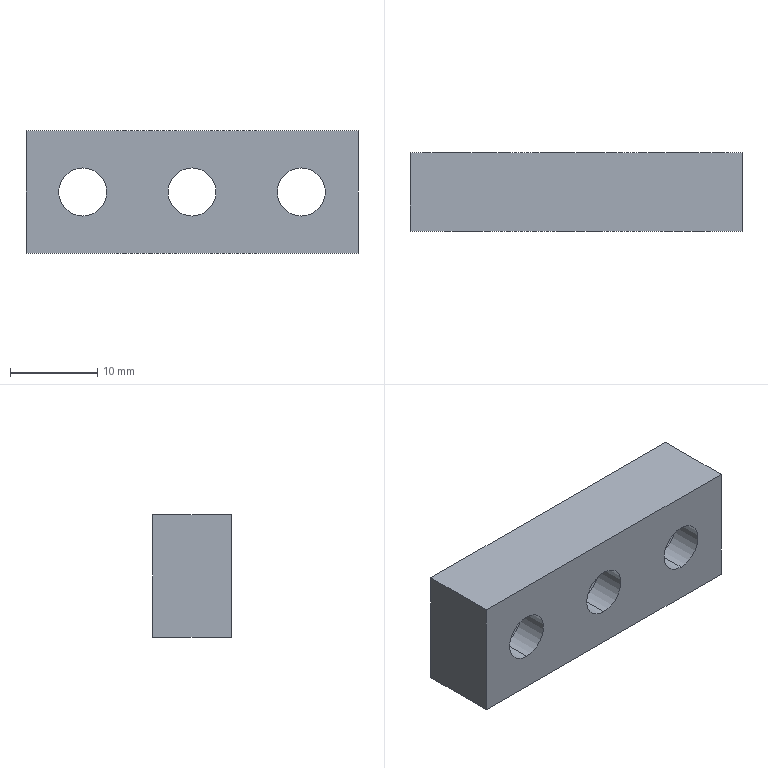Part | STEP file | 1 solid | 21 faces | box 38 x 9 x 14 mm | volume 3259 mm3 | cylinder 12 | plane 9 | commonest cylinder face diameters 5.5 x6 10 x6
STEP:
#1=CARTESIAN_POINT('',(0.,0.,0.));
#2=DIRECTION('',(0.,0.,1.));
#3=DIRECTION('',(1.,0.,0.));
#4=AXIS2_PLACEMENT_3D('',#1,#2,#3);
#5=CARTESIAN_POINT('',(0.,3.6,5.));
#6=VERTEX_POINT('',#5);
#7=CARTESIAN_POINT('',(0.,9.,5.));
#8=VERTEX_POINT('',#7);
#9=CARTESIAN_POINT('',(0.,9.,5.));
#10=DIRECTION('',(0.,1.,0.));
#11=VECTOR('',#10,1.);
#12=LINE('',#9,#11);
#13=CARTESIAN_POINT('',(0.,9.,0.));
#14=DIRECTION('',(0.,1.,0.));
#15=DIRECTION('',(0.,0.,1.));
#16=AXIS2_PLACEMENT_3D('',#13,#14,#15);
#17=CYLINDRICAL_SURFACE('',#16,5.);
#18=CARTESIAN_POINT('',(6.283,0.));
#19=DIRECTION('',(0.,1.));
#20=VECTOR('',#19,1.);
#21=LINE('',#18,#20);
#22=(GEOMETRIC_REPRESENTATION_CONTEXT(2)PARAMETRIC_REPRESENTATION_CONTEXT()REPRESENTATION_CONTEXT('',''));
#23=DEFINITIONAL_REPRESENTATION('',(#21),#22);
#24=PCURVE('',#17,#23);
#25=CARTESIAN_POINT('',(0.,9.,0.));
#26=DIRECTION('',(0.,1.,0.));
#27=DIRECTION('',(0.,0.,1.));
#28=AXIS2_PLACEMENT_3D('',#25,#26,#27);
#29=CYLINDRICAL_SURFACE('',#28,5.);
#30=CARTESIAN_POINT('',(0.,0.));
#31=DIRECTION('',(0.,1.));
#32=VECTOR('',#31,1.);
#33=LINE('',#30,#32);
#34=(GEOMETRIC_REPRESENTATION_CONTEXT(2)PARAMETRIC_REPRESENTATION_CONTEXT()REPRESENTATION_CONTEXT('',''));
#35=DEFINITIONAL_REPRESENTATION('',(#33),#34);
#36=PCURVE('',#29,#35);
#37=SURFACE_CURVE('',#12,(#24,#36),.PCURVE_S1.);
#38=EDGE_CURVE('',#6,#8,#37,.T.);
#39=ORIENTED_EDGE('',*,*,#38,.T.);
#40=CARTESIAN_POINT('',(0.,9.,-5.));
#41=VERTEX_POINT('',#40);
#42=CARTESIAN_POINT('',(0.,9.,0.));
#43=DIRECTION('',(0.,1.,0.));
#44=DIRECTION('',(0.,0.,1.));
#45=AXIS2_PLACEMENT_3D('',#42,#43,#44);
#46=CIRCLE('',#45,5.);
#47=CARTESIAN_POINT('',(0.,0.));
#48=DIRECTION('',(1.,0.));
#49=VECTOR('',#48,1.);
#50=LINE('',#47,#49);
#51=(GEOMETRIC_REPRESENTATION_CONTEXT(2)PARAMETRIC_REPRESENTATION_CONTEXT()REPRESENTATION_CONTEXT('',''));
#52=DEFINITIONAL_REPRESENTATION('',(#50),#51);
#53=PCURVE('',#17,#52);
#54=CARTESIAN_POINT('',(0.,9.,0.));
#55=DIRECTION('',(0.,1.,0.));
#56=DIRECTION('',(0.,0.,1.));
#57=AXIS2_PLACEMENT_3D('',#54,#55,#56);
#58=PLANE('',#57);
#59=CARTESIAN_POINT('',(0.,0.));
#60=DIRECTION('',(1.,0.));
#61=AXIS2_PLACEMENT_2D('',#59,#60);
#62=CIRCLE('',#61,5.);
#63=(GEOMETRIC_REPRESENTATION_CONTEXT(2)PARAMETRIC_REPRESENTATION_CONTEXT()REPRESENTATION_CONTEXT('',''));
#64=DEFINITIONAL_REPRESENTATION('',(#62),#63);
#65=PCURVE('',#58,#64);
#66=SURFACE_CURVE('',#46,(#53,#65),.PCURVE_S1.);
#67=EDGE_CURVE('',#41,#8,#66,.T.);
#68=ORIENTED_EDGE('',*,*,#67,.F.);
#69=CARTESIAN_POINT('',(0.,3.6,-5.));
#70=VERTEX_POINT('',#69);
#71=CARTESIAN_POINT('',(0.,9.,-5.));
#72=DIRECTION('',(0.,1.,0.));
#73=VECTOR('',#72,1.);
#74=LINE('',#71,#73);
#75=CARTESIAN_POINT('',(3.142,0.));
#76=DIRECTION('',(0.,1.));
#77=VECTOR('',#76,1.);
#78=LINE('',#75,#77);
#79=(GEOMETRIC_REPRESENTATION_CONTEXT(2)PARAMETRIC_REPRESENTATION_CONTEXT()REPRESENTATION_CONTEXT('',''));
#80=DEFINITIONAL_REPRESENTATION('',(#78),#79);
#81=PCURVE('',#17,#80);
#82=CARTESIAN_POINT('',(3.142,0.));
#83=DIRECTION('',(0.,1.));
#84=VECTOR('',#83,1.);
#85=LINE('',#82,#84);
#86=(GEOMETRIC_REPRESENTATION_CONTEXT(2)PARAMETRIC_REPRESENTATION_CONTEXT()REPRESENTATION_CONTEXT('',''));
#87=DEFINITIONAL_REPRESENTATION('',(#85),#86);
#88=PCURVE('',#29,#87);
#89=SURFACE_CURVE('',#74,(#81,#88),.PCURVE_S1.);
#90=EDGE_CURVE('',#70,#41,#89,.T.);
#91=ORIENTED_EDGE('',*,*,#90,.F.);
#92=CARTESIAN_POINT('',(0.,3.6,0.));
#93=DIRECTION('',(0.,1.,0.));
#94=DIRECTION('',(0.,0.,1.));
#95=AXIS2_PLACEMENT_3D('',#92,#93,#94);
#96=CIRCLE('',#95,5.);
#97=CARTESIAN_POINT('',(0.,-5.4));
#98=DIRECTION('',(1.,0.));
#99=VECTOR('',#98,1.);
#100=LINE('',#97,#99);
#101=(GEOMETRIC_REPRESENTATION_CONTEXT(2)PARAMETRIC_REPRESENTATION_CONTEXT()REPRESENTATION_CONTEXT('',''));
#102=DEFINITIONAL_REPRESENTATION('',(#100),#101);
#103=PCURVE('',#17,#102);
#104=CARTESIAN_POINT('',(2.75,3.6,0.));
#105=DIRECTION('',(0.,-1.,0.));
#106=DIRECTION('',(0.,0.,-1.));
#107=AXIS2_PLACEMENT_3D('',#104,#105,#106);
#108=PLANE('',#107);
#109=CARTESIAN_POINT('',(-5.,-2.75));
#110=CARTESIAN_POINT('',(-5.,5.91));
#111=CARTESIAN_POINT('',(2.5,1.58));
#112=CARTESIAN_POINT('',(10.,-2.75));
#113=CARTESIAN_POINT('',(2.5,-7.08));
#114=CARTESIAN_POINT('',(-5.,-11.41));
#115=CARTESIAN_POINT('',(-5.,-2.75));
#116=(BOUNDED_CURVE()B_SPLINE_CURVE(2,(#109,#110,#111,#112,#113,#114,#115),.UNSPECIFIED.,.T.,.F.)B_SPLINE_CURVE_WITH_KNOTS((1,2,2,2,2,1),(-2.094,0.,2.094,4.189,6.283,8.378),.UNSPECIFIED.)CURVE()GEOMETRIC_REPRESENTATION_ITEM()RATIONAL_B_SPLINE_CURVE((1.,0.5,1.,0.5,1.,0.5,1.))REPRESENTATION_ITEM(''));
#117=(GEOMETRIC_REPRESENTATION_CONTEXT(2)PARAMETRIC_REPRESENTATION_CONTEXT()REPRESENTATION_CONTEXT('',''));
#118=DEFINITIONAL_REPRESENTATION('',(#116),#117);
#119=PCURVE('',#108,#118);
#120=SURFACE_CURVE('',#96,(#103,#119),.PCURVE_S1.);
#121=EDGE_CURVE('',#70,#6,#120,.T.);
#122=ORIENTED_EDGE('',*,*,#121,.T.);
#123=EDGE_LOOP('',(#39,#68,#91,#122));
#124=FACE_BOUND('',#123,.F.);
#125=ADVANCED_FACE('',(#124),#17,.F.);
#126=CARTESIAN_POINT('',(0.,0.,2.75));
#127=VERTEX_POINT('',#126);
#128=CARTESIAN_POINT('',(0.,3.6,2.75));
#129=VERTEX_POINT('',#128);
#130=CARTESIAN_POINT('',(0.,9.,2.75));
#131=DIRECTION('',(0.,1.,0.));
#132=VECTOR('',#131,1.);
#133=LINE('',#130,#132);
#134=CARTESIAN_POINT('',(0.,9.,0.));
#135=DIRECTION('',(0.,1.,0.));
#136=DIRECTION('',(0.,0.,1.));
#137=AXIS2_PLACEMENT_3D('',#134,#135,#136);
#138=CYLINDRICAL_SURFACE('',#137,2.75);
#139=CARTESIAN_POINT('',(6.283,0.));
#140=DIRECTION('',(0.,1.));
#141=VECTOR('',#140,1.);
#142=LINE('',#139,#141);
#143=(GEOMETRIC_REPRESENTATION_CONTEXT(2)PARAMETRIC_REPRESENTATION_CONTEXT()REPRESENTATION_CONTEXT('',''));
#144=DEFINITIONAL_REPRESENTATION('',(#142),#143);
#145=PCURVE('',#138,#144);
#146=CARTESIAN_POINT('',(0.,9.,0.));
#147=DIRECTION('',(0.,1.,0.));
#148=DIRECTION('',(0.,0.,1.));
#149=AXIS2_PLACEMENT_3D('',#146,#147,#148);
#150=CYLINDRICAL_SURFACE('',#149,2.75);
#151=CARTESIAN_POINT('',(0.,0.));
#152=DIRECTION('',(0.,1.));
#153=VECTOR('',#152,1.);
#154=LINE('',#151,#153);
#155=(GEOMETRIC_REPRESENTATION_CONTEXT(2)PARAMETRIC_REPRESENTATION_CONTEXT()REPRESENTATION_CONTEXT('',''));
#156=DEFINITIONAL_REPRESENTATION('',(#154),#155);
#157=PCURVE('',#150,#156);
#158=SURFACE_CURVE('',#133,(#145,#157),.PCURVE_S1.);
#159=EDGE_CURVE('',#127,#129,#158,.T.);
#160=ORIENTED_EDGE('',*,*,#159,.T.);
#161=CARTESIAN_POINT('',(0.,3.6,-2.75));
#162=VERTEX_POINT('',#161);
#163=CARTESIAN_POINT('',(0.,3.6,0.));
#164=DIRECTION('',(0.,1.,0.));
#165=DIRECTION('',(0.,0.,1.));
#166=AXIS2_PLACEMENT_3D('',#163,#164,#165);
#167=CIRCLE('',#166,2.75);
#168=CARTESIAN_POINT('',(0.,-5.4));
#169=DIRECTION('',(1.,0.));
#170=VECTOR('',#169,1.);
#171=LINE('',#168,#170);
#172=(GEOMETRIC_REPRESENTATION_CONTEXT(2)PARAMETRIC_REPRESENTATION_CONTEXT()REPRESENTATION_CONTEXT('',''));
#173=DEFINITIONAL_REPRESENTATION('',(#171),#172);
#174=PCURVE('',#138,#173);
#175=CARTESIAN_POINT('',(-2.75,-2.75));
#176=CARTESIAN_POINT('',(-2.75,2.013));
#177=CARTESIAN_POINT('',(1.375,-0.3684));
#178=CARTESIAN_POINT('',(5.5,-2.75));
#179=CARTESIAN_POINT('',(1.375,-5.132));
#180=CARTESIAN_POINT('',(-2.75,-7.513));
#181=CARTESIAN_POINT('',(-2.75,-2.75));
#182=(BOUNDED_CURVE()B_SPLINE_CURVE(2,(#175,#176,#177,#178,#179,#180,#181),.UNSPECIFIED.,.T.,.F.)B_SPLINE_CURVE_WITH_KNOTS((1,2,2,2,2,1),(-2.094,0.,2.094,4.189,6.283,8.378),.UNSPECIFIED.)CURVE()GEOMETRIC_REPRESENTATION_ITEM()RATIONAL_B_SPLINE_CURVE((1.,0.5,1.,0.5,1.,0.5,1.))REPRESENTATION_ITEM(''));
#183=(GEOMETRIC_REPRESENTATION_CONTEXT(2)PARAMETRIC_REPRESENTATION_CONTEXT()REPRESENTATION_CONTEXT('',''));
#184=DEFINITIONAL_REPRESENTATION('',(#182),#183);
#185=PCURVE('',#108,#184);
#186=SURFACE_CURVE('',#167,(#174,#185),.PCURVE_S1.);
#187=EDGE_CURVE('',#162,#129,#186,.T.);
#188=ORIENTED_EDGE('',*,*,#187,.F.);
#189=CARTESIAN_POINT('',(0.,0.,-2.75));
#190=VERTEX_POINT('',#189);
#191=CARTESIAN_POINT('',(0.,9.,-2.75));
#192=DIRECTION('',(0.,1.,0.));
#193=VECTOR('',#192,1.);
#194=LINE('',#191,#193);
#195=CARTESIAN_POINT('',(3.142,0.));
#196=DIRECTION('',(0.,1.));
#197=VECTOR('',#196,1.);
#198=LINE('',#195,#197);
#199=(GEOMETRIC_REPRESENTATION_CONTEXT(2)PARAMETRIC_REPRESENTATION_CONTEXT()REPRESENTATION_CONTEXT('',''));
#200=DEFINITIONAL_REPRESENTATION('',(#198),#199);
#201=PCURVE('',#138,#200);
#202=CARTESIAN_POINT('',(3.142,0.));
#203=DIRECTION('',(0.,1.));
#204=VECTOR('',#203,1.);
#205=LINE('',#202,#204);
#206=(GEOMETRIC_REPRESENTATION_CONTEXT(2)PARAMETRIC_REPRESENTATION_CONTEXT()REPRESENTATION_CONTEXT('',''));
#207=DEFINITIONAL_REPRESENTATION('',(#205),#206);
#208=PCURVE('',#150,#207);
#209=SURFACE_CURVE('',#194,(#201,#208),.PCURVE_S1.);
#210=EDGE_CURVE('',#190,#162,#209,.T.);
#211=ORIENTED_EDGE('',*,*,#210,.F.);
#212=CARTESIAN_POINT('',(0.,0.,0.));
#213=DIRECTION('',(0.,1.,0.));
#214=DIRECTION('',(0.,0.,1.));
#215=AXIS2_PLACEMENT_3D('',#212,#213,#214);
#216=CIRCLE('',#215,2.75);
#217=CARTESIAN_POINT('',(0.,-9.));
#218=DIRECTION('',(1.,0.));
#219=VECTOR('',#218,1.);
#220=LINE('',#217,#219);
#221=(GEOMETRIC_REPRESENTATION_CONTEXT(2)PARAMETRIC_REPRESENTATION_CONTEXT()REPRESENTATION_CONTEXT('',''));
#222=DEFINITIONAL_REPRESENTATION('',(#220),#221);
#223=PCURVE('',#138,#222);
#224=CARTESIAN_POINT('',(0.,0.,0.));
#225=DIRECTION('',(0.,1.,0.));
#226=DIRECTION('',(0.,0.,1.));
#227=AXIS2_PLACEMENT_3D('',#224,#225,#226);
#228=PLANE('',#227);
#229=CARTESIAN_POINT('',(0.,0.));
#230=DIRECTION('',(1.,0.));
#231=AXIS2_PLACEMENT_2D('',#229,#230);
#232=CIRCLE('',#231,2.75);
#233=(GEOMETRIC_REPRESENTATION_CONTEXT(2)PARAMETRIC_REPRESENTATION_CONTEXT()REPRESENTATION_CONTEXT('',''));
#234=DEFINITIONAL_REPRESENTATION('',(#232),#233);
#235=PCURVE('',#228,#234);
#236=SURFACE_CURVE('',#216,(#223,#235),.PCURVE_S1.);
#237=EDGE_CURVE('',#190,#127,#236,.T.);
#238=ORIENTED_EDGE('',*,*,#237,.T.);
#239=EDGE_LOOP('',(#160,#188,#211,#238));
#240=FACE_BOUND('',#239,.F.);
#241=ADVANCED_FACE('',(#240),#138,.F.);
#242=CARTESIAN_POINT('',(-12.5,3.6,5.));
#243=VERTEX_POINT('',#242);
#244=CARTESIAN_POINT('',(-12.5,9.,5.));
#245=VERTEX_POINT('',#244);
#246=CARTESIAN_POINT('',(-12.5,9.,5.));
#247=DIRECTION('',(0.,1.,0.));
#248=VECTOR('',#247,1.);
#249=LINE('',#246,#248);
#250=CARTESIAN_POINT('',(-12.5,9.,0.));
#251=DIRECTION('',(0.,1.,0.));
#252=DIRECTION('',(0.,0.,1.));
#253=AXIS2_PLACEMENT_3D('',#250,#251,#252);
#254=CYLINDRICAL_SURFACE('',#253,5.);
#255=CARTESIAN_POINT('',(6.283,0.));
#256=DIRECTION('',(0.,1.));
#257=VECTOR('',#256,1.);
#258=LINE('',#255,#257);
#259=(GEOMETRIC_REPRESENTATION_CONTEXT(2)PARAMETRIC_REPRESENTATION_CONTEXT()REPRESENTATION_CONTEXT('',''));
#260=DEFINITIONAL_REPRESENTATION('',(#258),#259);
#261=PCURVE('',#254,#260);
#262=CARTESIAN_POINT('',(-12.5,9.,0.));
#263=DIRECTION('',(0.,1.,0.));
#264=DIRECTION('',(0.,0.,1.));
#265=AXIS2_PLACEMENT_3D('',#262,#263,#264);
#266=CYLINDRICAL_SURFACE('',#265,5.);
#267=CARTESIAN_POINT('',(0.,0.));
#268=DIRECTION('',(0.,1.));
#269=VECTOR('',#268,1.);
#270=LINE('',#267,#269);
#271=(GEOMETRIC_REPRESENTATION_CONTEXT(2)PARAMETRIC_REPRESENTATION_CONTEXT()REPRESENTATION_CONTEXT('',''));
#272=DEFINITIONAL_REPRESENTATION('',(#270),#271);
#273=PCURVE('',#266,#272);
#274=SURFACE_CURVE('',#249,(#261,#273),.PCURVE_S1.);
#275=EDGE_CURVE('',#243,#245,#274,.T.);
#276=ORIENTED_EDGE('',*,*,#275,.T.);
#277=CARTESIAN_POINT('',(-12.5,9.,-5.));
#278=VERTEX_POINT('',#277);
#279=CARTESIAN_POINT('',(-12.5,9.,0.));
#280=DIRECTION('',(0.,1.,0.));
#281=DIRECTION('',(0.,0.,1.));
#282=AXIS2_PLACEMENT_3D('',#279,#280,#281);
#283=CIRCLE('',#282,5.);
#284=CARTESIAN_POINT('',(0.,0.));
#285=DIRECTION('',(1.,0.));
#286=VECTOR('',#285,1.);
#287=LINE('',#284,#286);
#288=(GEOMETRIC_REPRESENTATION_CONTEXT(2)PARAMETRIC_REPRESENTATION_CONTEXT()REPRESENTATION_CONTEXT('',''));
#289=DEFINITIONAL_REPRESENTATION('',(#287),#288);
#290=PCURVE('',#254,#289);
#291=CARTESIAN_POINT('',(0.,-12.5));
#292=DIRECTION('',(1.,0.));
#293=AXIS2_PLACEMENT_2D('',#291,#292);
#294=CIRCLE('',#293,5.);
#295=(GEOMETRIC_REPRESENTATION_CONTEXT(2)PARAMETRIC_REPRESENTATION_CONTEXT()REPRESENTATION_CONTEXT('',''));
#296=DEFINITIONAL_REPRESENTATION('',(#294),#295);
#297=PCURVE('',#58,#296);
#298=SURFACE_CURVE('',#283,(#290,#297),.PCURVE_S1.);
#299=EDGE_CURVE('',#278,#245,#298,.T.);
#300=ORIENTED_EDGE('',*,*,#299,.F.);
#301=CARTESIAN_POINT('',(-12.5,3.6,-5.));
#302=VERTEX_POINT('',#301);
#303=CARTESIAN_POINT('',(-12.5,9.,-5.));
#304=DIRECTION('',(0.,1.,0.));
#305=VECTOR('',#304,1.);
#306=LINE('',#303,#305);
#307=CARTESIAN_POINT('',(3.142,0.));
#308=DIRECTION('',(0.,1.));
#309=VECTOR('',#308,1.);
#310=LINE('',#307,#309);
#311=(GEOMETRIC_REPRESENTATION_CONTEXT(2)PARAMETRIC_REPRESENTATION_CONTEXT()REPRESENTATION_CONTEXT('',''));
#312=DEFINITIONAL_REPRESENTATION('',(#310),#311);
#313=PCURVE('',#254,#312);
#314=CARTESIAN_POINT('',(3.142,0.));
#315=DIRECTION('',(0.,1.));
#316=VECTOR('',#315,1.);
#317=LINE('',#314,#316);
#318=(GEOMETRIC_REPRESENTATION_CONTEXT(2)PARAMETRIC_REPRESENTATION_CONTEXT()REPRESENTATION_CONTEXT('',''));
#319=DEFINITIONAL_REPRESENTATION('',(#317),#318);
#320=PCURVE('',#266,#319);
#321=SURFACE_CURVE('',#306,(#313,#320),.PCURVE_S1.);
#322=EDGE_CURVE('',#302,#278,#321,.T.);
#323=ORIENTED_EDGE('',*,*,#322,.F.);
#324=CARTESIAN_POINT('',(-12.5,3.6,0.));
#325=DIRECTION('',(0.,1.,0.));
#326=DIRECTION('',(0.,0.,1.));
#327=AXIS2_PLACEMENT_3D('',#324,#325,#326);
#328=CIRCLE('',#327,5.);
#329=CARTESIAN_POINT('',(0.,-5.4));
#330=DIRECTION('',(1.,0.));
#331=VECTOR('',#330,1.);
#332=LINE('',#329,#331);
#333=(GEOMETRIC_REPRESENTATION_CONTEXT(2)PARAMETRIC_REPRESENTATION_CONTEXT()REPRESENTATION_CONTEXT('',''));
#334=DEFINITIONAL_REPRESENTATION('',(#332),#333);
#335=PCURVE('',#254,#334);
#336=CARTESIAN_POINT('',(-9.75,3.6,0.));
#337=DIRECTION('',(0.,-1.,0.));
#338=DIRECTION('',(0.,0.,-1.));
#339=AXIS2_PLACEMENT_3D('',#336,#337,#338);
#340=PLANE('',#339);
#341=CARTESIAN_POINT('',(-5.,-2.75));
#342=CARTESIAN_POINT('',(-5.,5.91));
#343=CARTESIAN_POINT('',(2.5,1.58));
#344=CARTESIAN_POINT('',(10.,-2.75));
#345=CARTESIAN_POINT('',(2.5,-7.08));
#346=CARTESIAN_POINT('',(-5.,-11.41));
#347=CARTESIAN_POINT('',(-5.,-2.75));
#348=(BOUNDED_CURVE()B_SPLINE_CURVE(2,(#341,#342,#343,#344,#345,#346,#347),.UNSPECIFIED.,.T.,.F.)B_SPLINE_CURVE_WITH_KNOTS((1,2,2,2,2,1),(-2.094,0.,2.094,4.189,6.283,8.378),.UNSPECIFIED.)CURVE()GEOMETRIC_REPRESENTATION_ITEM()RATIONAL_B_SPLINE_CURVE((1.,0.5,1.,0.5,1.,0.5,1.))REPRESENTATION_ITEM(''));
#349=(GEOMETRIC_REPRESENTATION_CONTEXT(2)PARAMETRIC_REPRESENTATION_CONTEXT()REPRESENTATION_CONTEXT('',''));
#350=DEFINITIONAL_REPRESENTATION('',(#348),#349);
#351=PCURVE('',#340,#350);
#352=SURFACE_CURVE('',#328,(#335,#351),.PCURVE_S1.);
#353=EDGE_CURVE('',#302,#243,#352,.T.);
#354=ORIENTED_EDGE('',*,*,#353,.T.);
#355=EDGE_LOOP('',(#276,#300,#323,#354));
#356=FACE_BOUND('',#355,.F.);
#357=ADVANCED_FACE('',(#356),#254,.F.);
#358=CARTESIAN_POINT('',(-12.5,0.,2.75));
#359=VERTEX_POINT('',#358);
#360=CARTESIAN_POINT('',(-12.5,3.6,2.75));
#361=VERTEX_POINT('',#360);
#362=CARTESIAN_POINT('',(-12.5,9.,2.75));
#363=DIRECTION('',(0.,1.,0.));
#364=VECTOR('',#363,1.);
#365=LINE('',#362,#364);
#366=CARTESIAN_POINT('',(-12.5,9.,0.));
#367=DIRECTION('',(0.,1.,0.));
#368=DIRECTION('',(0.,0.,1.));
#369=AXIS2_PLACEMENT_3D('',#366,#367,#368);
#370=CYLINDRICAL_SURFACE('',#369,2.75);
#371=CARTESIAN_POINT('',(6.283,0.));
#372=DIRECTION('',(0.,1.));
#373=VECTOR('',#372,1.);
#374=LINE('',#371,#373);
#375=(GEOMETRIC_REPRESENTATION_CONTEXT(2)PARAMETRIC_REPRESENTATION_CONTEXT()REPRESENTATION_CONTEXT('',''));
#376=DEFINITIONAL_REPRESENTATION('',(#374),#375);
#377=PCURVE('',#370,#376);
#378=CARTESIAN_POINT('',(-12.5,9.,0.));
#379=DIRECTION('',(0.,1.,0.));
#380=DIRECTION('',(0.,0.,1.));
#381=AXIS2_PLACEMENT_3D('',#378,#379,#380);
#382=CYLINDRICAL_SURFACE('',#381,2.75);
#383=CARTESIAN_POINT('',(0.,0.));
#384=DIRECTION('',(0.,1.));
#385=VECTOR('',#384,1.);
#386=LINE('',#383,#385);
#387=(GEOMETRIC_REPRESENTATION_CONTEXT(2)PARAMETRIC_REPRESENTATION_CONTEXT()REPRESENTATION_CONTEXT('',''));
#388=DEFINITIONAL_REPRESENTATION('',(#386),#387);
#389=PCURVE('',#382,#388);
#390=SURFACE_CURVE('',#365,(#377,#389),.PCURVE_S1.);
#391=EDGE_CURVE('',#359,#361,#390,.T.);
#392=ORIENTED_EDGE('',*,*,#391,.T.);
#393=CARTESIAN_POINT('',(-12.5,3.6,-2.75));
#394=VERTEX_POINT('',#393);
#395=CARTESIAN_POINT('',(-12.5,3.6,0.));
#396=DIRECTION('',(0.,1.,0.));
#397=DIRECTION('',(0.,0.,1.));
#398=AXIS2_PLACEMENT_3D('',#395,#396,#397);
#399=CIRCLE('',#398,2.75);
#400=CARTESIAN_POINT('',(0.,-5.4));
#401=DIRECTION('',(1.,0.));
#402=VECTOR('',#401,1.);
#403=LINE('',#400,#402);
#404=(GEOMETRIC_REPRESENTATION_CONTEXT(2)PARAMETRIC_REPRESENTATION_CONTEXT()REPRESENTATION_CONTEXT('',''));
#405=DEFINITIONAL_REPRESENTATION('',(#403),#404);
#406=PCURVE('',#370,#405);
#407=CARTESIAN_POINT('',(-2.75,-2.75));
#408=CARTESIAN_POINT('',(-2.75,2.013));
#409=CARTESIAN_POINT('',(1.375,-0.3684));
#410=CARTESIAN_POINT('',(5.5,-2.75));
#411=CARTESIAN_POINT('',(1.375,-5.132));
#412=CARTESIAN_POINT('',(-2.75,-7.513));
#413=CARTESIAN_POINT('',(-2.75,-2.75));
#414=(BOUNDED_CURVE()B_SPLINE_CURVE(2,(#407,#408,#409,#410,#411,#412,#413),.UNSPECIFIED.,.T.,.F.)B_SPLINE_CURVE_WITH_KNOTS((1,2,2,2,2,1),(-2.094,0.,2.094,4.189,6.283,8.378),.UNSPECIFIED.)CURVE()GEOMETRIC_REPRESENTATION_ITEM()RATIONAL_B_SPLINE_CURVE((1.,0.5,1.,0.5,1.,0.5,1.))REPRESENTATION_ITEM(''));
#415=(GEOMETRIC_REPRESENTATION_CONTEXT(2)PARAMETRIC_REPRESENTATION_CONTEXT()REPRESENTATION_CONTEXT('',''));
#416=DEFINITIONAL_REPRESENTATION('',(#414),#415);
#417=PCURVE('',#340,#416);
#418=SURFACE_CURVE('',#399,(#406,#417),.PCURVE_S1.);
#419=EDGE_CURVE('',#394,#361,#418,.T.);
#420=ORIENTED_EDGE('',*,*,#419,.F.);
#421=CARTESIAN_POINT('',(-12.5,0.,-2.75));
#422=VERTEX_POINT('',#421);
#423=CARTESIAN_POINT('',(-12.5,9.,-2.75));
#424=DIRECTION('',(0.,1.,0.));
#425=VECTOR('',#424,1.);
#426=LINE('',#423,#425);
#427=CARTESIAN_POINT('',(3.142,0.));
#428=DIRECTION('',(0.,1.));
#429=VECTOR('',#428,1.);
#430=LINE('',#427,#429);
#431=(GEOMETRIC_REPRESENTATION_CONTEXT(2)PARAMETRIC_REPRESENTATION_CONTEXT()REPRESENTATION_CONTEXT('',''));
#432=DEFINITIONAL_REPRESENTATION('',(#430),#431);
#433=PCURVE('',#370,#432);
#434=CARTESIAN_POINT('',(3.142,0.));
#435=DIRECTION('',(0.,1.));
#436=VECTOR('',#435,1.);
#437=LINE('',#434,#436);
#438=(GEOMETRIC_REPRESENTATION_CONTEXT(2)PARAMETRIC_REPRESENTATION_CONTEXT()REPRESENTATION_CONTEXT('',''));
#439=DEFINITIONAL_REPRESENTATION('',(#437),#438);
#440=PCURVE('',#382,#439);
#441=SURFACE_CURVE('',#426,(#433,#440),.PCURVE_S1.);
#442=EDGE_CURVE('',#422,#394,#441,.T.);
#443=ORIENTED_EDGE('',*,*,#442,.F.);
#444=CARTESIAN_POINT('',(-12.5,0.,0.));
#445=DIRECTION('',(0.,1.,0.));
#446=DIRECTION('',(0.,0.,1.));
#447=AXIS2_PLACEMENT_3D('',#444,#445,#446);
#448=CIRCLE('',#447,2.75);
#449=CARTESIAN_POINT('',(0.,-9.));
#450=DIRECTION('',(1.,0.));
#451=VECTOR('',#450,1.);
#452=LINE('',#449,#451);
#453=(GEOMETRIC_REPRESENTATION_CONTEXT(2)PARAMETRIC_REPRESENTATION_CONTEXT()REPRESENTATION_CONTEXT('',''));
#454=DEFINITIONAL_REPRESENTATION('',(#452),#453);
#455=PCURVE('',#370,#454);
#456=CARTESIAN_POINT('',(0.,-12.5));
#457=DIRECTION('',(1.,0.));
#458=AXIS2_PLACEMENT_2D('',#456,#457);
#459=CIRCLE('',#458,2.75);
#460=(GEOMETRIC_REPRESENTATION_CONTEXT(2)PARAMETRIC_REPRESENTATION_CONTEXT()REPRESENTATION_CONTEXT('',''));
#461=DEFINITIONAL_REPRESENTATION('',(#459),#460);
#462=PCURVE('',#228,#461);
#463=SURFACE_CURVE('',#448,(#455,#462),.PCURVE_S1.);
#464=EDGE_CURVE('',#422,#359,#463,.T.);
#465=ORIENTED_EDGE('',*,*,#464,.T.);
#466=EDGE_LOOP('',(#392,#420,#443,#465));
#467=FACE_BOUND('',#466,.F.);
#468=ADVANCED_FACE('',(#467),#370,.F.);
#469=CARTESIAN_POINT('',(12.5,3.6,5.));
#470=VERTEX_POINT('',#469);
#471=CARTESIAN_POINT('',(12.5,9.,5.));
#472=VERTEX_POINT('',#471);
#473=CARTESIAN_POINT('',(12.5,9.,5.));
#474=DIRECTION('',(0.,1.,0.));
#475=VECTOR('',#474,1.);
#476=LINE('',#473,#475);
#477=CARTESIAN_POINT('',(12.5,9.,0.));
#478=DIRECTION('',(0.,1.,0.));
#479=DIRECTION('',(0.,0.,1.));
#480=AXIS2_PLACEMENT_3D('',#477,#478,#479);
#481=CYLINDRICAL_SURFACE('',#480,5.);
#482=CARTESIAN_POINT('',(6.283,0.));
#483=DIRECTION('',(0.,1.));
#484=VECTOR('',#483,1.);
#485=LINE('',#482,#484);
#486=(GEOMETRIC_REPRESENTATION_CONTEXT(2)PARAMETRIC_REPRESENTATION_CONTEXT()REPRESENTATION_CONTEXT('',''));
#487=DEFINITIONAL_REPRESENTATION('',(#485),#486);
#488=PCURVE('',#481,#487);
#489=CARTESIAN_POINT('',(12.5,9.,0.));
#490=DIRECTION('',(0.,1.,0.));
#491=DIRECTION('',(0.,0.,1.));
#492=AXIS2_PLACEMENT_3D('',#489,#490,#491);
#493=CYLINDRICAL_SURFACE('',#492,5.);
#494=CARTESIAN_POINT('',(0.,0.));
#495=DIRECTION('',(0.,1.));
#496=VECTOR('',#495,1.);
#497=LINE('',#494,#496);
#498=(GEOMETRIC_REPRESENTATION_CONTEXT(2)PARAMETRIC_REPRESENTATION_CONTEXT()REPRESENTATION_CONTEXT('',''));
#499=DEFINITIONAL_REPRESENTATION('',(#497),#498);
#500=PCURVE('',#493,#499);
#501=SURFACE_CURVE('',#476,(#488,#500),.PCURVE_S1.);
#502=EDGE_CURVE('',#470,#472,#501,.T.);
#503=ORIENTED_EDGE('',*,*,#502,.T.);
#504=CARTESIAN_POINT('',(12.5,9.,-5.));
#505=VERTEX_POINT('',#504);
#506=CARTESIAN_POINT('',(12.5,9.,0.));
#507=DIRECTION('',(0.,1.,0.));
#508=DIRECTION('',(0.,0.,1.));
#509=AXIS2_PLACEMENT_3D('',#506,#507,#508);
#510=CIRCLE('',#509,5.);
#511=CARTESIAN_POINT('',(0.,0.));
#512=DIRECTION('',(1.,0.));
#513=VECTOR('',#512,1.);
#514=LINE('',#511,#513);
#515=(GEOMETRIC_REPRESENTATION_CONTEXT(2)PARAMETRIC_REPRESENTATION_CONTEXT()REPRESENTATION_CONTEXT('',''));
#516=DEFINITIONAL_REPRESENTATION('',(#514),#515);
#517=PCURVE('',#481,#516);
#518=CARTESIAN_POINT('',(0.,12.5));
#519=DIRECTION('',(1.,0.));
#520=AXIS2_PLACEMENT_2D('',#518,#519);
#521=CIRCLE('',#520,5.);
#522=(GEOMETRIC_REPRESENTATION_CONTEXT(2)PARAMETRIC_REPRESENTATION_CONTEXT()REPRESENTATION_CONTEXT('',''));
#523=DEFINITIONAL_REPRESENTATION('',(#521),#522);
#524=PCURVE('',#58,#523);
#525=SURFACE_CURVE('',#510,(#517,#524),.PCURVE_S1.);
#526=EDGE_CURVE('',#505,#472,#525,.T.);
#527=ORIENTED_EDGE('',*,*,#526,.F.);
#528=CARTESIAN_POINT('',(12.5,3.6,-5.));
#529=VERTEX_POINT('',#528);
#530=CARTESIAN_POINT('',(12.5,9.,-5.));
#531=DIRECTION('',(0.,1.,0.));
#532=VECTOR('',#531,1.);
#533=LINE('',#530,#532);
#534=CARTESIAN_POINT('',(3.142,0.));
#535=DIRECTION('',(0.,1.));
#536=VECTOR('',#535,1.);
#537=LINE('',#534,#536);
#538=(GEOMETRIC_REPRESENTATION_CONTEXT(2)PARAMETRIC_REPRESENTATION_CONTEXT()REPRESENTATION_CONTEXT('',''));
#539=DEFINITIONAL_REPRESENTATION('',(#537),#538);
#540=PCURVE('',#481,#539);
#541=CARTESIAN_POINT('',(3.142,0.));
#542=DIRECTION('',(0.,1.));
#543=VECTOR('',#542,1.);
#544=LINE('',#541,#543);
#545=(GEOMETRIC_REPRESENTATION_CONTEXT(2)PARAMETRIC_REPRESENTATION_CONTEXT()REPRESENTATION_CONTEXT('',''));
#546=DEFINITIONAL_REPRESENTATION('',(#544),#545);
#547=PCURVE('',#493,#546);
#548=SURFACE_CURVE('',#533,(#540,#547),.PCURVE_S1.);
#549=EDGE_CURVE('',#529,#505,#548,.T.);
#550=ORIENTED_EDGE('',*,*,#549,.F.);
#551=CARTESIAN_POINT('',(12.5,3.6,0.));
#552=DIRECTION('',(0.,1.,0.));
#553=DIRECTION('',(0.,0.,1.));
#554=AXIS2_PLACEMENT_3D('',#551,#552,#553);
#555=CIRCLE('',#554,5.);
#556=CARTESIAN_POINT('',(0.,-5.4));
#557=DIRECTION('',(1.,0.));
#558=VECTOR('',#557,1.);
#559=LINE('',#556,#558);
#560=(GEOMETRIC_REPRESENTATION_CONTEXT(2)PARAMETRIC_REPRESENTATION_CONTEXT()REPRESENTATION_CONTEXT('',''));
#561=DEFINITIONAL_REPRESENTATION('',(#559),#560);
#562=PCURVE('',#481,#561);
#563=CARTESIAN_POINT('',(15.25,3.6,0.));
#564=DIRECTION('',(0.,-1.,0.));
#565=DIRECTION('',(0.,0.,-1.));
#566=AXIS2_PLACEMENT_3D('',#563,#564,#565);
#567=PLANE('',#566);
#568=CARTESIAN_POINT('',(-5.,-2.75));
#569=CARTESIAN_POINT('',(-5.,5.91));
#570=CARTESIAN_POINT('',(2.5,1.58));
#571=CARTESIAN_POINT('',(10.,-2.75));
#572=CARTESIAN_POINT('',(2.5,-7.08));
#573=CARTESIAN_POINT('',(-5.,-11.41));
#574=CARTESIAN_POINT('',(-5.,-2.75));
#575=(BOUNDED_CURVE()B_SPLINE_CURVE(2,(#568,#569,#570,#571,#572,#573,#574),.UNSPECIFIED.,.T.,.F.)B_SPLINE_CURVE_WITH_KNOTS((1,2,2,2,2,1),(-2.094,0.,2.094,4.189,6.283,8.378),.UNSPECIFIED.)CURVE()GEOMETRIC_REPRESENTATION_ITEM()RATIONAL_B_SPLINE_CURVE((1.,0.5,1.,0.5,1.,0.5,1.))REPRESENTATION_ITEM(''));
#576=(GEOMETRIC_REPRESENTATION_CONTEXT(2)PARAMETRIC_REPRESENTATION_CONTEXT()REPRESENTATION_CONTEXT('',''));
#577=DEFINITIONAL_REPRESENTATION('',(#575),#576);
#578=PCURVE('',#567,#577);
#579=SURFACE_CURVE('',#555,(#562,#578),.PCURVE_S1.);
#580=EDGE_CURVE('',#529,#470,#579,.T.);
#581=ORIENTED_EDGE('',*,*,#580,.T.);
#582=EDGE_LOOP('',(#503,#527,#550,#581));
#583=FACE_BOUND('',#582,.F.);
#584=ADVANCED_FACE('',(#583),#481,.F.);
#585=CARTESIAN_POINT('',(12.5,0.,2.75));
#586=VERTEX_POINT('',#585);
#587=CARTESIAN_POINT('',(12.5,3.6,2.75));
#588=VERTEX_POINT('',#587);
#589=CARTESIAN_POINT('',(12.5,9.,2.75));
#590=DIRECTION('',(0.,1.,0.));
#591=VECTOR('',#590,1.);
#592=LINE('',#589,#591);
#593=CARTESIAN_POINT('',(12.5,9.,0.));
#594=DIRECTION('',(0.,1.,0.));
#595=DIRECTION('',(0.,0.,1.));
#596=AXIS2_PLACEMENT_3D('',#593,#594,#595);
#597=CYLINDRICAL_SURFACE('',#596,2.75);
#598=CARTESIAN_POINT('',(6.283,0.));
#599=DIRECTION('',(0.,1.));
#600=VECTOR('',#599,1.);
#601=LINE('',#598,#600);
#602=(GEOMETRIC_REPRESENTATION_CONTEXT(2)PARAMETRIC_REPRESENTATION_CONTEXT()REPRESENTATION_CONTEXT('',''));
#603=DEFINITIONAL_REPRESENTATION('',(#601),#602);
#604=PCURVE('',#597,#603);
#605=CARTESIAN_POINT('',(12.5,9.,0.));
#606=DIRECTION('',(0.,1.,0.));
#607=DIRECTION('',(0.,0.,1.));
#608=AXIS2_PLACEMENT_3D('',#605,#606,#607);
#609=CYLINDRICAL_SURFACE('',#608,2.75);
#610=CARTESIAN_POINT('',(0.,0.));
#611=DIRECTION('',(0.,1.));
#612=VECTOR('',#611,1.);
#613=LINE('',#610,#612);
#614=(GEOMETRIC_REPRESENTATION_CONTEXT(2)PARAMETRIC_REPRESENTATION_CONTEXT()REPRESENTATION_CONTEXT('',''));
#615=DEFINITIONAL_REPRESENTATION('',(#613),#614);
#616=PCURVE('',#609,#615);
#617=SURFACE_CURVE('',#592,(#604,#616),.PCURVE_S1.);
#618=EDGE_CURVE('',#586,#588,#617,.T.);
#619=ORIENTED_EDGE('',*,*,#618,.T.);
#620=CARTESIAN_POINT('',(12.5,3.6,-2.75));
#621=VERTEX_POINT('',#620);
#622=CARTESIAN_POINT('',(12.5,3.6,0.));
#623=DIRECTION('',(0.,1.,0.));
#624=DIRECTION('',(0.,0.,1.));
#625=AXIS2_PLACEMENT_3D('',#622,#623,#624);
#626=CIRCLE('',#625,2.75);
#627=CARTESIAN_POINT('',(0.,-5.4));
#628=DIRECTION('',(1.,0.));
#629=VECTOR('',#628,1.);
#630=LINE('',#627,#629);
#631=(GEOMETRIC_REPRESENTATION_CONTEXT(2)PARAMETRIC_REPRESENTATION_CONTEXT()REPRESENTATION_CONTEXT('',''));
#632=DEFINITIONAL_REPRESENTATION('',(#630),#631);
#633=PCURVE('',#597,#632);
#634=CARTESIAN_POINT('',(-2.75,-2.75));
#635=CARTESIAN_POINT('',(-2.75,2.013));
#636=CARTESIAN_POINT('',(1.375,-0.3684));
#637=CARTESIAN_POINT('',(5.5,-2.75));
#638=CARTESIAN_POINT('',(1.375,-5.132));
#639=CARTESIAN_POINT('',(-2.75,-7.513));
#640=CARTESIAN_POINT('',(-2.75,-2.75));
#641=(BOUNDED_CURVE()B_SPLINE_CURVE(2,(#634,#635,#636,#637,#638,#639,#640),.UNSPECIFIED.,.T.,.F.)B_SPLINE_CURVE_WITH_KNOTS((1,2,2,2,2,1),(-2.094,0.,2.094,4.189,6.283,8.378),.UNSPECIFIED.)CURVE()GEOMETRIC_REPRESENTATION_ITEM()RATIONAL_B_SPLINE_CURVE((1.,0.5,1.,0.5,1.,0.5,1.))REPRESENTATION_ITEM(''));
#642=(GEOMETRIC_REPRESENTATION_CONTEXT(2)PARAMETRIC_REPRESENTATION_CONTEXT()REPRESENTATION_CONTEXT('',''));
#643=DEFINITIONAL_REPRESENTATION('',(#641),#642);
#644=PCURVE('',#567,#643);
#645=SURFACE_CURVE('',#626,(#633,#644),.PCURVE_S1.);
#646=EDGE_CURVE('',#621,#588,#645,.T.);
#647=ORIENTED_EDGE('',*,*,#646,.F.);
#648=CARTESIAN_POINT('',(12.5,0.,-2.75));
#649=VERTEX_POINT('',#648);
#650=CARTESIAN_POINT('',(12.5,9.,-2.75));
#651=DIRECTION('',(0.,1.,0.));
#652=VECTOR('',#651,1.);
#653=LINE('',#650,#652);
#654=CARTESIAN_POINT('',(3.142,0.));
#655=DIRECTION('',(0.,1.));
#656=VECTOR('',#655,1.);
#657=LINE('',#654,#656);
#658=(GEOMETRIC_REPRESENTATION_CONTEXT(2)PARAMETRIC_REPRESENTATION_CONTEXT()REPRESENTATION_CONTEXT('',''));
#659=DEFINITIONAL_REPRESENTATION('',(#657),#658);
#660=PCURVE('',#597,#659);
#661=CARTESIAN_POINT('',(3.142,0.));
#662=DIRECTION('',(0.,1.));
#663=VECTOR('',#662,1.);
#664=LINE('',#661,#663);
#665=(GEOMETRIC_REPRESENTATION_CONTEXT(2)PARAMETRIC_REPRESENTATION_CONTEXT()REPRESENTATION_CONTEXT('',''));
#666=DEFINITIONAL_REPRESENTATION('',(#664),#665);
#667=PCURVE('',#609,#666);
#668=SURFACE_CURVE('',#653,(#660,#667),.PCURVE_S1.);
#669=EDGE_CURVE('',#649,#621,#668,.T.);
#670=ORIENTED_EDGE('',*,*,#669,.F.);
#671=CARTESIAN_POINT('',(12.5,0.,0.));
#672=DIRECTION('',(0.,1.,0.));
#673=DIRECTION('',(0.,0.,1.));
#674=AXIS2_PLACEMENT_3D('',#671,#672,#673);
#675=CIRCLE('',#674,2.75);
#676=CARTESIAN_POINT('',(0.,-9.));
#677=DIRECTION('',(1.,0.));
#678=VECTOR('',#677,1.);
#679=LINE('',#676,#678);
#680=(GEOMETRIC_REPRESENTATION_CONTEXT(2)PARAMETRIC_REPRESENTATION_CONTEXT()REPRESENTATION_CONTEXT('',''));
#681=DEFINITIONAL_REPRESENTATION('',(#679),#680);
#682=PCURVE('',#597,#681);
#683=CARTESIAN_POINT('',(0.,12.5));
#684=DIRECTION('',(1.,0.));
#685=AXIS2_PLACEMENT_2D('',#683,#684);
#686=CIRCLE('',#685,2.75);
#687=(GEOMETRIC_REPRESENTATION_CONTEXT(2)PARAMETRIC_REPRESENTATION_CONTEXT()REPRESENTATION_CONTEXT('',''));
#688=DEFINITIONAL_REPRESENTATION('',(#686),#687);
#689=PCURVE('',#228,#688);
#690=SURFACE_CURVE('',#675,(#682,#689),.PCURVE_S1.);
#691=EDGE_CURVE('',#649,#586,#690,.T.);
#692=ORIENTED_EDGE('',*,*,#691,.T.);
#693=EDGE_LOOP('',(#619,#647,#670,#692));
#694=FACE_BOUND('',#693,.F.);
#695=ADVANCED_FACE('',(#694),#597,.F.);
#696=CARTESIAN_POINT('',(-19.,0.,-7.));
#697=VERTEX_POINT('',#696);
#698=CARTESIAN_POINT('',(-19.,0.,7.));
#699=VERTEX_POINT('',#698);
#700=CARTESIAN_POINT('',(-19.,0.,7.));
#701=DIRECTION('',(0.,0.,1.));
#702=VECTOR('',#701,1.);
#703=LINE('',#700,#702);
#704=CARTESIAN_POINT('',(-19.,9.,7.));
#705=DIRECTION('',(1.,0.,0.));
#706=DIRECTION('',(0.,0.,-1.));
#707=AXIS2_PLACEMENT_3D('',#704,#705,#706);
#708=PLANE('',#707);
#709=CARTESIAN_POINT('',(0.,-9.));
#710=DIRECTION('',(-1.,0.));
#711=VECTOR('',#710,1.);
#712=LINE('',#709,#711);
#713=(GEOMETRIC_REPRESENTATION_CONTEXT(2)PARAMETRIC_REPRESENTATION_CONTEXT()REPRESENTATION_CONTEXT('',''));
#714=DEFINITIONAL_REPRESENTATION('',(#712),#713);
#715=PCURVE('',#708,#714);
#716=CARTESIAN_POINT('',(7.,-19.));
#717=DIRECTION('',(1.,0.));
#718=VECTOR('',#717,1.);
#719=LINE('',#716,#718);
#720=(GEOMETRIC_REPRESENTATION_CONTEXT(2)PARAMETRIC_REPRESENTATION_CONTEXT()REPRESENTATION_CONTEXT('',''));
#721=DEFINITIONAL_REPRESENTATION('',(#719),#720);
#722=PCURVE('',#228,#721);
#723=SURFACE_CURVE('',#703,(#715,#722),.PCURVE_S1.);
#724=EDGE_CURVE('',#697,#699,#723,.T.);
#725=ORIENTED_EDGE('',*,*,#724,.T.);
#726=CARTESIAN_POINT('',(-19.,9.,7.));
#727=VERTEX_POINT('',#726);
#728=CARTESIAN_POINT('',(-19.,9.,7.));
#729=DIRECTION('',(0.,-1.,0.));
#730=VECTOR('',#729,1.);
#731=LINE('',#728,#730);
#732=CARTESIAN_POINT('',(0.,0.));
#733=DIRECTION('',(0.,-1.));
#734=VECTOR('',#733,1.);
#735=LINE('',#732,#734);
#736=(GEOMETRIC_REPRESENTATION_CONTEXT(2)PARAMETRIC_REPRESENTATION_CONTEXT()REPRESENTATION_CONTEXT('',''));
#737=DEFINITIONAL_REPRESENTATION('',(#735),#736);
#738=PCURVE('',#708,#737);
#739=CARTESIAN_POINT('',(19.,9.,7.));
#740=DIRECTION('',(0.,0.,-1.));
#741=DIRECTION('',(-1.,0.,0.));
#742=AXIS2_PLACEMENT_3D('',#739,#740,#741);
#743=PLANE('',#742);
#744=CARTESIAN_POINT('',(38.,0.));
#745=DIRECTION('',(0.,-1.));
#746=VECTOR('',#745,1.);
#747=LINE('',#744,#746);
#748=(GEOMETRIC_REPRESENTATION_CONTEXT(2)PARAMETRIC_REPRESENTATION_CONTEXT()REPRESENTATION_CONTEXT('',''));
#749=DEFINITIONAL_REPRESENTATION('',(#747),#748);
#750=PCURVE('',#743,#749);
#751=SURFACE_CURVE('',#731,(#738,#750),.PCURVE_S1.);
#752=EDGE_CURVE('',#727,#699,#751,.T.);
#753=ORIENTED_EDGE('',*,*,#752,.F.);
#754=CARTESIAN_POINT('',(-19.,9.,-7.));
#755=VERTEX_POINT('',#754);
#756=CARTESIAN_POINT('',(-19.,9.,7.));
#757=DIRECTION('',(0.,0.,1.));
#758=VECTOR('',#757,1.);
#759=LINE('',#756,#758);
#760=CARTESIAN_POINT('',(0.,0.));
#761=DIRECTION('',(-1.,0.));
#762=VECTOR('',#761,1.);
#763=LINE('',#760,#762);
#764=(GEOMETRIC_REPRESENTATION_CONTEXT(2)PARAMETRIC_REPRESENTATION_CONTEXT()REPRESENTATION_CONTEXT('',''));
#765=DEFINITIONAL_REPRESENTATION('',(#763),#764);
#766=PCURVE('',#708,#765);
#767=CARTESIAN_POINT('',(7.,-19.));
#768=DIRECTION('',(1.,0.));
#769=VECTOR('',#768,1.);
#770=LINE('',#767,#769);
#771=(GEOMETRIC_REPRESENTATION_CONTEXT(2)PARAMETRIC_REPRESENTATION_CONTEXT()REPRESENTATION_CONTEXT('',''));
#772=DEFINITIONAL_REPRESENTATION('',(#770),#771);
#773=PCURVE('',#58,#772);
#774=SURFACE_CURVE('',#759,(#766,#773),.PCURVE_S1.);
#775=EDGE_CURVE('',#755,#727,#774,.T.);
#776=ORIENTED_EDGE('',*,*,#775,.F.);
#777=CARTESIAN_POINT('',(-19.,9.,-7.));
#778=DIRECTION('',(0.,-1.,0.));
#779=VECTOR('',#778,1.);
#780=LINE('',#777,#779);
#781=CARTESIAN_POINT('',(14.,0.));
#782=DIRECTION('',(0.,-1.));
#783=VECTOR('',#782,1.);
#784=LINE('',#781,#783);
#785=(GEOMETRIC_REPRESENTATION_CONTEXT(2)PARAMETRIC_REPRESENTATION_CONTEXT()REPRESENTATION_CONTEXT('',''));
#786=DEFINITIONAL_REPRESENTATION('',(#784),#785);
#787=PCURVE('',#708,#786);
#788=CARTESIAN_POINT('',(19.,9.,-7.));
#789=DIRECTION('',(0.,0.,1.));
#790=DIRECTION('',(1.,0.,0.));
#791=AXIS2_PLACEMENT_3D('',#788,#789,#790);
#792=PLANE('',#791);
#793=CARTESIAN_POINT('',(-38.,0.));
#794=DIRECTION('',(0.,-1.));
#795=VECTOR('',#794,1.);
#796=LINE('',#793,#795);
#797=(GEOMETRIC_REPRESENTATION_CONTEXT(2)PARAMETRIC_REPRESENTATION_CONTEXT()REPRESENTATION_CONTEXT('',''));
#798=DEFINITIONAL_REPRESENTATION('',(#796),#797);
#799=PCURVE('',#792,#798);
#800=SURFACE_CURVE('',#780,(#787,#799),.PCURVE_S1.);
#801=EDGE_CURVE('',#755,#697,#800,.T.);
#802=ORIENTED_EDGE('',*,*,#801,.T.);
#803=EDGE_LOOP('',(#725,#753,#776,#802));
#804=FACE_BOUND('',#803,.T.);
#805=ADVANCED_FACE('',(#804),#708,.F.);
#806=CARTESIAN_POINT('',(19.,0.,7.));
#807=VERTEX_POINT('',#806);
#808=CARTESIAN_POINT('',(19.,0.,7.));
#809=DIRECTION('',(1.,0.,0.));
#810=VECTOR('',#809,1.);
#811=LINE('',#808,#810);
#812=CARTESIAN_POINT('',(0.,-9.));
#813=DIRECTION('',(-1.,0.));
#814=VECTOR('',#813,1.);
#815=LINE('',#812,#814);
#816=(GEOMETRIC_REPRESENTATION_CONTEXT(2)PARAMETRIC_REPRESENTATION_CONTEXT()REPRESENTATION_CONTEXT('',''));
#817=DEFINITIONAL_REPRESENTATION('',(#815),#816);
#818=PCURVE('',#743,#817);
#819=CARTESIAN_POINT('',(7.,19.));
#820=DIRECTION('',(0.,1.));
#821=VECTOR('',#820,1.);
#822=LINE('',#819,#821);
#823=(GEOMETRIC_REPRESENTATION_CONTEXT(2)PARAMETRIC_REPRESENTATION_CONTEXT()REPRESENTATION_CONTEXT('',''));
#824=DEFINITIONAL_REPRESENTATION('',(#822),#823);
#825=PCURVE('',#228,#824);
#826=SURFACE_CURVE('',#811,(#818,#825),.PCURVE_S1.);
#827=EDGE_CURVE('',#699,#807,#826,.T.);
#828=ORIENTED_EDGE('',*,*,#827,.T.);
#829=CARTESIAN_POINT('',(19.,9.,7.));
#830=VERTEX_POINT('',#829);
#831=CARTESIAN_POINT('',(19.,9.,7.));
#832=DIRECTION('',(0.,-1.,0.));
#833=VECTOR('',#832,1.);
#834=LINE('',#831,#833);
#835=CARTESIAN_POINT('',(0.,0.));
#836=DIRECTION('',(0.,-1.));
#837=VECTOR('',#836,1.);
#838=LINE('',#835,#837);
#839=(GEOMETRIC_REPRESENTATION_CONTEXT(2)PARAMETRIC_REPRESENTATION_CONTEXT()REPRESENTATION_CONTEXT('',''));
#840=DEFINITIONAL_REPRESENTATION('',(#838),#839);
#841=PCURVE('',#743,#840);
#842=CARTESIAN_POINT('',(19.,9.,7.));
#843=DIRECTION('',(-1.,0.,0.));
#844=DIRECTION('',(0.,0.,1.));
#845=AXIS2_PLACEMENT_3D('',#842,#843,#844);
#846=PLANE('',#845);
#847=CARTESIAN_POINT('',(0.,0.));
#848=DIRECTION('',(0.,-1.));
#849=VECTOR('',#848,1.);
#850=LINE('',#847,#849);
#851=(GEOMETRIC_REPRESENTATION_CONTEXT(2)PARAMETRIC_REPRESENTATION_CONTEXT()REPRESENTATION_CONTEXT('',''));
#852=DEFINITIONAL_REPRESENTATION('',(#850),#851);
#853=PCURVE('',#846,#852);
#854=SURFACE_CURVE('',#834,(#841,#853),.PCURVE_S1.);
#855=EDGE_CURVE('',#830,#807,#854,.T.);
#856=ORIENTED_EDGE('',*,*,#855,.F.);
#857=CARTESIAN_POINT('',(19.,9.,7.));
#858=DIRECTION('',(1.,0.,0.));
#859=VECTOR('',#858,1.);
#860=LINE('',#857,#859);
#861=CARTESIAN_POINT('',(0.,0.));
#862=DIRECTION('',(-1.,0.));
#863=VECTOR('',#862,1.);
#864=LINE('',#861,#863);
#865=(GEOMETRIC_REPRESENTATION_CONTEXT(2)PARAMETRIC_REPRESENTATION_CONTEXT()REPRESENTATION_CONTEXT('',''));
#866=DEFINITIONAL_REPRESENTATION('',(#864),#865);
#867=PCURVE('',#743,#866);
#868=CARTESIAN_POINT('',(7.,19.));
#869=DIRECTION('',(0.,1.));
#870=VECTOR('',#869,1.);
#871=LINE('',#868,#870);
#872=(GEOMETRIC_REPRESENTATION_CONTEXT(2)PARAMETRIC_REPRESENTATION_CONTEXT()REPRESENTATION_CONTEXT('',''));
#873=DEFINITIONAL_REPRESENTATION('',(#871),#872);
#874=PCURVE('',#58,#873);
#875=SURFACE_CURVE('',#860,(#867,#874),.PCURVE_S1.);
#876=EDGE_CURVE('',#727,#830,#875,.T.);
#877=ORIENTED_EDGE('',*,*,#876,.F.);
#878=ORIENTED_EDGE('',*,*,#752,.T.);
#879=EDGE_LOOP('',(#828,#856,#877,#878));
#880=FACE_BOUND('',#879,.T.);
#881=ADVANCED_FACE('',(#880),#743,.F.);
#882=CARTESIAN_POINT('',(19.,0.,-7.));
#883=VERTEX_POINT('',#882);
#884=CARTESIAN_POINT('',(19.,0.,7.));
#885=DIRECTION('',(0.,0.,-1.));
#886=VECTOR('',#885,1.);
#887=LINE('',#884,#886);
#888=CARTESIAN_POINT('',(0.,-9.));
#889=DIRECTION('',(-1.,0.));
#890=VECTOR('',#889,1.);
#891=LINE('',#888,#890);
#892=(GEOMETRIC_REPRESENTATION_CONTEXT(2)PARAMETRIC_REPRESENTATION_CONTEXT()REPRESENTATION_CONTEXT('',''));
#893=DEFINITIONAL_REPRESENTATION('',(#891),#892);
#894=PCURVE('',#846,#893);
#895=CARTESIAN_POINT('',(7.,19.));
#896=DIRECTION('',(-1.,0.));
#897=VECTOR('',#896,1.);
#898=LINE('',#895,#897);
#899=(GEOMETRIC_REPRESENTATION_CONTEXT(2)PARAMETRIC_REPRESENTATION_CONTEXT()REPRESENTATION_CONTEXT('',''));
#900=DEFINITIONAL_REPRESENTATION('',(#898),#899);
#901=PCURVE('',#228,#900);
#902=SURFACE_CURVE('',#887,(#894,#901),.PCURVE_S1.);
#903=EDGE_CURVE('',#807,#883,#902,.T.);
#904=ORIENTED_EDGE('',*,*,#903,.T.);
#905=CARTESIAN_POINT('',(19.,9.,-7.));
#906=VERTEX_POINT('',#905);
#907=CARTESIAN_POINT('',(19.,9.,-7.));
#908=DIRECTION('',(0.,-1.,0.));
#909=VECTOR('',#908,1.);
#910=LINE('',#907,#909);
#911=CARTESIAN_POINT('',(-14.,0.));
#912=DIRECTION('',(0.,-1.));
#913=VECTOR('',#912,1.);
#914=LINE('',#911,#913);
#915=(GEOMETRIC_REPRESENTATION_CONTEXT(2)PARAMETRIC_REPRESENTATION_CONTEXT()REPRESENTATION_CONTEXT('',''));
#916=DEFINITIONAL_REPRESENTATION('',(#914),#915);
#917=PCURVE('',#846,#916);
#918=CARTESIAN_POINT('',(0.,0.));
#919=DIRECTION('',(0.,-1.));
#920=VECTOR('',#919,1.);
#921=LINE('',#918,#920);
#922=(GEOMETRIC_REPRESENTATION_CONTEXT(2)PARAMETRIC_REPRESENTATION_CONTEXT()REPRESENTATION_CONTEXT('',''));
#923=DEFINITIONAL_REPRESENTATION('',(#921),#922);
#924=PCURVE('',#792,#923);
#925=SURFACE_CURVE('',#910,(#917,#924),.PCURVE_S1.);
#926=EDGE_CURVE('',#906,#883,#925,.T.);
#927=ORIENTED_EDGE('',*,*,#926,.F.);
#928=CARTESIAN_POINT('',(19.,9.,7.));
#929=DIRECTION('',(0.,0.,-1.));
#930=VECTOR('',#929,1.);
#931=LINE('',#928,#930);
#932=CARTESIAN_POINT('',(0.,0.));
#933=DIRECTION('',(-1.,0.));
#934=VECTOR('',#933,1.);
#935=LINE('',#932,#934);
#936=(GEOMETRIC_REPRESENTATION_CONTEXT(2)PARAMETRIC_REPRESENTATION_CONTEXT()REPRESENTATION_CONTEXT('',''));
#937=DEFINITIONAL_REPRESENTATION('',(#935),#936);
#938=PCURVE('',#846,#937);
#939=CARTESIAN_POINT('',(7.,19.));
#940=DIRECTION('',(-1.,0.));
#941=VECTOR('',#940,1.);
#942=LINE('',#939,#941);
#943=(GEOMETRIC_REPRESENTATION_CONTEXT(2)PARAMETRIC_REPRESENTATION_CONTEXT()REPRESENTATION_CONTEXT('',''));
#944=DEFINITIONAL_REPRESENTATION('',(#942),#943);
#945=PCURVE('',#58,#944);
#946=SURFACE_CURVE('',#931,(#938,#945),.PCURVE_S1.);
#947=EDGE_CURVE('',#830,#906,#946,.T.);
#948=ORIENTED_EDGE('',*,*,#947,.F.);
#949=ORIENTED_EDGE('',*,*,#855,.T.);
#950=EDGE_LOOP('',(#904,#927,#948,#949));
#951=FACE_BOUND('',#950,.T.);
#952=ADVANCED_FACE('',(#951),#846,.F.);
#953=CARTESIAN_POINT('',(19.,0.,-7.));
#954=DIRECTION('',(-1.,0.,0.));
#955=VECTOR('',#954,1.);
#956=LINE('',#953,#955);
#957=CARTESIAN_POINT('',(0.,-9.));
#958=DIRECTION('',(-1.,0.));
#959=VECTOR('',#958,1.);
#960=LINE('',#957,#959);
#961=(GEOMETRIC_REPRESENTATION_CONTEXT(2)PARAMETRIC_REPRESENTATION_CONTEXT()REPRESENTATION_CONTEXT('',''));
#962=DEFINITIONAL_REPRESENTATION('',(#960),#961);
#963=PCURVE('',#792,#962);
#964=CARTESIAN_POINT('',(-7.,19.));
#965=DIRECTION('',(0.,-1.));
#966=VECTOR('',#965,1.);
#967=LINE('',#964,#966);
#968=(GEOMETRIC_REPRESENTATION_CONTEXT(2)PARAMETRIC_REPRESENTATION_CONTEXT()REPRESENTATION_CONTEXT('',''));
#969=DEFINITIONAL_REPRESENTATION('',(#967),#968);
#970=PCURVE('',#228,#969);
#971=SURFACE_CURVE('',#956,(#963,#970),.PCURVE_S1.);
#972=EDGE_CURVE('',#883,#697,#971,.T.);
#973=ORIENTED_EDGE('',*,*,#972,.T.);
#974=ORIENTED_EDGE('',*,*,#801,.F.);
#975=CARTESIAN_POINT('',(19.,9.,-7.));
#976=DIRECTION('',(-1.,0.,0.));
#977=VECTOR('',#976,1.);
#978=LINE('',#975,#977);
#979=CARTESIAN_POINT('',(0.,0.));
#980=DIRECTION('',(-1.,0.));
#981=VECTOR('',#980,1.);
#982=LINE('',#979,#981);
#983=(GEOMETRIC_REPRESENTATION_CONTEXT(2)PARAMETRIC_REPRESENTATION_CONTEXT()REPRESENTATION_CONTEXT('',''));
#984=DEFINITIONAL_REPRESENTATION('',(#982),#983);
#985=PCURVE('',#792,#984);
#986=CARTESIAN_POINT('',(-7.,19.));
#987=DIRECTION('',(0.,-1.));
#988=VECTOR('',#987,1.);
#989=LINE('',#986,#988);
#990=(GEOMETRIC_REPRESENTATION_CONTEXT(2)PARAMETRIC_REPRESENTATION_CONTEXT()REPRESENTATION_CONTEXT('',''));
#991=DEFINITIONAL_REPRESENTATION('',(#989),#990);
#992=PCURVE('',#58,#991);
#993=SURFACE_CURVE('',#978,(#985,#992),.PCURVE_S1.);
#994=EDGE_CURVE('',#906,#755,#993,.T.);
#995=ORIENTED_EDGE('',*,*,#994,.F.);
#996=ORIENTED_EDGE('',*,*,#926,.T.);
#997=EDGE_LOOP('',(#973,#974,#995,#996));
#998=FACE_BOUND('',#997,.T.);
#999=ADVANCED_FACE('',(#998),#792,.F.);
#1000=CARTESIAN_POINT('',(0.,9.,0.));
#1001=DIRECTION('',(0.,1.,0.));
#1002=DIRECTION('',(0.,0.,1.));
#1003=AXIS2_PLACEMENT_3D('',#1000,#1001,#1002);
#1004=CIRCLE('',#1003,5.);
#1005=CARTESIAN_POINT('',(0.,0.));
#1006=DIRECTION('',(1.,0.));
#1007=AXIS2_PLACEMENT_2D('',#1005,#1006);
#1008=CIRCLE('',#1007,5.);
#1009=(GEOMETRIC_REPRESENTATION_CONTEXT(2)PARAMETRIC_REPRESENTATION_CONTEXT()REPRESENTATION_CONTEXT('',''));
#1010=DEFINITIONAL_REPRESENTATION('',(#1008),#1009);
#1011=PCURVE('',#58,#1010);
#1012=CARTESIAN_POINT('',(0.,0.));
#1013=DIRECTION('',(1.,0.));
#1014=VECTOR('',#1013,1.);
#1015=LINE('',#1012,#1014);
#1016=(GEOMETRIC_REPRESENTATION_CONTEXT(2)PARAMETRIC_REPRESENTATION_CONTEXT()REPRESENTATION_CONTEXT('',''));
#1017=DEFINITIONAL_REPRESENTATION('',(#1015),#1016);
#1018=PCURVE('',#29,#1017);
#1019=SURFACE_CURVE('',#1004,(#1011,#1018),.PCURVE_S1.);
#1020=EDGE_CURVE('',#8,#41,#1019,.T.);
#1021=ORIENTED_EDGE('',*,*,#1020,.F.);
#1022=ORIENTED_EDGE('',*,*,#67,.F.);
#1023=EDGE_LOOP('',(#1021,#1022));
#1024=FACE_BOUND('',#1023,.T.);
#1025=CARTESIAN_POINT('',(-12.5,9.,0.));
#1026=DIRECTION('',(0.,1.,0.));
#1027=DIRECTION('',(0.,0.,1.));
#1028=AXIS2_PLACEMENT_3D('',#1025,#1026,#1027);
#1029=CIRCLE('',#1028,5.);
#1030=CARTESIAN_POINT('',(0.,-12.5));
#1031=DIRECTION('',(1.,0.));
#1032=AXIS2_PLACEMENT_2D('',#1030,#1031);
#1033=CIRCLE('',#1032,5.);
#1034=(GEOMETRIC_REPRESENTATION_CONTEXT(2)PARAMETRIC_REPRESENTATION_CONTEXT()REPRESENTATION_CONTEXT('',''));
#1035=DEFINITIONAL_REPRESENTATION('',(#1033),#1034);
#1036=PCURVE('',#58,#1035);
#1037=CARTESIAN_POINT('',(0.,0.));
#1038=DIRECTION('',(1.,0.));
#1039=VECTOR('',#1038,1.);
#1040=LINE('',#1037,#1039);
#1041=(GEOMETRIC_REPRESENTATION_CONTEXT(2)PARAMETRIC_REPRESENTATION_CONTEXT()REPRESENTATION_CONTEXT('',''));
#1042=DEFINITIONAL_REPRESENTATION('',(#1040),#1041);
#1043=PCURVE('',#266,#1042);
#1044=SURFACE_CURVE('',#1029,(#1036,#1043),.PCURVE_S1.);
#1045=EDGE_CURVE('',#245,#278,#1044,.T.);
#1046=ORIENTED_EDGE('',*,*,#1045,.F.);
#1047=ORIENTED_EDGE('',*,*,#299,.F.);
#1048=EDGE_LOOP('',(#1046,#1047));
#1049=FACE_BOUND('',#1048,.T.);
#1050=CARTESIAN_POINT('',(12.5,9.,0.));
#1051=DIRECTION('',(0.,1.,0.));
#1052=DIRECTION('',(0.,0.,1.));
#1053=AXIS2_PLACEMENT_3D('',#1050,#1051,#1052);
#1054=CIRCLE('',#1053,5.);
#1055=CARTESIAN_POINT('',(0.,12.5));
#1056=DIRECTION('',(1.,0.));
#1057=AXIS2_PLACEMENT_2D('',#1055,#1056);
#1058=CIRCLE('',#1057,5.);
#1059=(GEOMETRIC_REPRESENTATION_CONTEXT(2)PARAMETRIC_REPRESENTATION_CONTEXT()REPRESENTATION_CONTEXT('',''));
#1060=DEFINITIONAL_REPRESENTATION('',(#1058),#1059);
#1061=PCURVE('',#58,#1060);
#1062=CARTESIAN_POINT('',(0.,0.));
#1063=DIRECTION('',(1.,0.));
#1064=VECTOR('',#1063,1.);
#1065=LINE('',#1062,#1064);
#1066=(GEOMETRIC_REPRESENTATION_CONTEXT(2)PARAMETRIC_REPRESENTATION_CONTEXT()REPRESENTATION_CONTEXT('',''));
#1067=DEFINITIONAL_REPRESENTATION('',(#1065),#1066);
#1068=PCURVE('',#493,#1067);
#1069=SURFACE_CURVE('',#1054,(#1061,#1068),.PCURVE_S1.);
#1070=EDGE_CURVE('',#472,#505,#1069,.T.);
#1071=ORIENTED_EDGE('',*,*,#1070,.F.);
#1072=ORIENTED_EDGE('',*,*,#526,.F.);
#1073=EDGE_LOOP('',(#1071,#1072));
#1074=FACE_BOUND('',#1073,.T.);
#1075=ORIENTED_EDGE('',*,*,#775,.T.);
#1076=ORIENTED_EDGE('',*,*,#876,.T.);
#1077=ORIENTED_EDGE('',*,*,#947,.T.);
#1078=ORIENTED_EDGE('',*,*,#994,.T.);
#1079=EDGE_LOOP('',(#1075,#1076,#1077,#1078));
#1080=FACE_BOUND('',#1079,.T.);
#1081=ADVANCED_FACE('',(#1024,#1049,#1074,#1080),#58,.T.);
#1082=CARTESIAN_POINT('',(0.,0.,0.));
#1083=DIRECTION('',(0.,1.,0.));
#1084=DIRECTION('',(0.,0.,1.));
#1085=AXIS2_PLACEMENT_3D('',#1082,#1083,#1084);
#1086=CIRCLE('',#1085,2.75);
#1087=CARTESIAN_POINT('',(0.,0.));
#1088=DIRECTION('',(1.,0.));
#1089=AXIS2_PLACEMENT_2D('',#1087,#1088);
#1090=CIRCLE('',#1089,2.75);
#1091=(GEOMETRIC_REPRESENTATION_CONTEXT(2)PARAMETRIC_REPRESENTATION_CONTEXT()REPRESENTATION_CONTEXT('',''));
#1092=DEFINITIONAL_REPRESENTATION('',(#1090),#1091);
#1093=PCURVE('',#228,#1092);
#1094=CARTESIAN_POINT('',(0.,-9.));
#1095=DIRECTION('',(1.,0.));
#1096=VECTOR('',#1095,1.);
#1097=LINE('',#1094,#1096);
#1098=(GEOMETRIC_REPRESENTATION_CONTEXT(2)PARAMETRIC_REPRESENTATION_CONTEXT()REPRESENTATION_CONTEXT('',''));
#1099=DEFINITIONAL_REPRESENTATION('',(#1097),#1098);
#1100=PCURVE('',#150,#1099);
#1101=SURFACE_CURVE('',#1086,(#1093,#1100),.PCURVE_S1.);
#1102=EDGE_CURVE('',#127,#190,#1101,.T.);
#1103=ORIENTED_EDGE('',*,*,#1102,.T.);
#1104=ORIENTED_EDGE('',*,*,#237,.T.);
#1105=EDGE_LOOP('',(#1103,#1104));
#1106=FACE_BOUND('',#1105,.T.);
#1107=CARTESIAN_POINT('',(-12.5,0.,0.));
#1108=DIRECTION('',(0.,1.,0.));
#1109=DIRECTION('',(0.,0.,1.));
#1110=AXIS2_PLACEMENT_3D('',#1107,#1108,#1109);
#1111=CIRCLE('',#1110,2.75);
#1112=CARTESIAN_POINT('',(0.,-12.5));
#1113=DIRECTION('',(1.,0.));
#1114=AXIS2_PLACEMENT_2D('',#1112,#1113);
#1115=CIRCLE('',#1114,2.75);
#1116=(GEOMETRIC_REPRESENTATION_CONTEXT(2)PARAMETRIC_REPRESENTATION_CONTEXT()REPRESENTATION_CONTEXT('',''));
#1117=DEFINITIONAL_REPRESENTATION('',(#1115),#1116);
#1118=PCURVE('',#228,#1117);
#1119=CARTESIAN_POINT('',(0.,-9.));
#1120=DIRECTION('',(1.,0.));
#1121=VECTOR('',#1120,1.);
#1122=LINE('',#1119,#1121);
#1123=(GEOMETRIC_REPRESENTATION_CONTEXT(2)PARAMETRIC_REPRESENTATION_CONTEXT()REPRESENTATION_CONTEXT('',''));
#1124=DEFINITIONAL_REPRESENTATION('',(#1122),#1123);
#1125=PCURVE('',#382,#1124);
#1126=SURFACE_CURVE('',#1111,(#1118,#1125),.PCURVE_S1.);
#1127=EDGE_CURVE('',#359,#422,#1126,.T.);
#1128=ORIENTED_EDGE('',*,*,#1127,.T.);
#1129=ORIENTED_EDGE('',*,*,#464,.T.);
#1130=EDGE_LOOP('',(#1128,#1129));
#1131=FACE_BOUND('',#1130,.T.);
#1132=CARTESIAN_POINT('',(12.5,0.,0.));
#1133=DIRECTION('',(0.,1.,0.));
#1134=DIRECTION('',(0.,0.,1.));
#1135=AXIS2_PLACEMENT_3D('',#1132,#1133,#1134);
#1136=CIRCLE('',#1135,2.75);
#1137=CARTESIAN_POINT('',(0.,12.5));
#1138=DIRECTION('',(1.,0.));
#1139=AXIS2_PLACEMENT_2D('',#1137,#1138);
#1140=CIRCLE('',#1139,2.75);
#1141=(GEOMETRIC_REPRESENTATION_CONTEXT(2)PARAMETRIC_REPRESENTATION_CONTEXT()REPRESENTATION_CONTEXT('',''));
#1142=DEFINITIONAL_REPRESENTATION('',(#1140),#1141);
#1143=PCURVE('',#228,#1142);
#1144=CARTESIAN_POINT('',(0.,-9.));
#1145=DIRECTION('',(1.,0.));
#1146=VECTOR('',#1145,1.);
#1147=LINE('',#1144,#1146);
#1148=(GEOMETRIC_REPRESENTATION_CONTEXT(2)PARAMETRIC_REPRESENTATION_CONTEXT()REPRESENTATION_CONTEXT('',''));
#1149=DEFINITIONAL_REPRESENTATION('',(#1147),#1148);
#1150=PCURVE('',#609,#1149);
#1151=SURFACE_CURVE('',#1136,(#1143,#1150),.PCURVE_S1.);
#1152=EDGE_CURVE('',#586,#649,#1151,.T.);
#1153=ORIENTED_EDGE('',*,*,#1152,.T.);
#1154=ORIENTED_EDGE('',*,*,#691,.T.);
#1155=EDGE_LOOP('',(#1153,#1154));
#1156=FACE_BOUND('',#1155,.T.);
#1157=ORIENTED_EDGE('',*,*,#724,.F.);
#1158=ORIENTED_EDGE('',*,*,#972,.F.);
#1159=ORIENTED_EDGE('',*,*,#903,.F.);
#1160=ORIENTED_EDGE('',*,*,#827,.F.);
#1161=EDGE_LOOP('',(#1157,#1158,#1159,#1160));
#1162=FACE_BOUND('',#1161,.T.);
#1163=ADVANCED_FACE('',(#1106,#1131,#1156,#1162),#228,.F.);
#1164=CARTESIAN_POINT('',(12.5,3.6,0.));
#1165=DIRECTION('',(0.,1.,0.));
#1166=DIRECTION('',(0.,0.,1.));
#1167=AXIS2_PLACEMENT_3D('',#1164,#1165,#1166);
#1168=CIRCLE('',#1167,2.75);
#1169=CARTESIAN_POINT('',(0.,-5.4));
#1170=DIRECTION('',(1.,0.));
#1171=VECTOR('',#1170,1.);
#1172=LINE('',#1169,#1171);
#1173=(GEOMETRIC_REPRESENTATION_CONTEXT(2)PARAMETRIC_REPRESENTATION_CONTEXT()REPRESENTATION_CONTEXT('',''));
#1174=DEFINITIONAL_REPRESENTATION('',(#1172),#1173);
#1175=PCURVE('',#609,#1174);
#1176=CARTESIAN_POINT('',(-2.75,-2.75));
#1177=CARTESIAN_POINT('',(-2.75,2.013));
#1178=CARTESIAN_POINT('',(1.375,-0.3684));
#1179=CARTESIAN_POINT('',(5.5,-2.75));
#1180=CARTESIAN_POINT('',(1.375,-5.132));
#1181=CARTESIAN_POINT('',(-2.75,-7.513));
#1182=CARTESIAN_POINT('',(-2.75,-2.75));
#1183=(BOUNDED_CURVE()B_SPLINE_CURVE(2,(#1176,#1177,#1178,#1179,#1180,#1181,#1182),.UNSPECIFIED.,.T.,.F.)B_SPLINE_CURVE_WITH_KNOTS((1,2,2,2,2,1),(-2.094,0.,2.094,4.189,6.283,8.378),.UNSPECIFIED.)CURVE()GEOMETRIC_REPRESENTATION_ITEM()RATIONAL_B_SPLINE_CURVE((1.,0.5,1.,0.5,1.,0.5,1.))REPRESENTATION_ITEM(''));
#1184=(GEOMETRIC_REPRESENTATION_CONTEXT(2)PARAMETRIC_REPRESENTATION_CONTEXT()REPRESENTATION_CONTEXT('',''));
#1185=DEFINITIONAL_REPRESENTATION('',(#1183),#1184);
#1186=PCURVE('',#567,#1185);
#1187=SURFACE_CURVE('',#1168,(#1175,#1186),.PCURVE_S1.);
#1188=EDGE_CURVE('',#588,#621,#1187,.T.);
#1189=ORIENTED_EDGE('',*,*,#1188,.F.);
#1190=ORIENTED_EDGE('',*,*,#618,.F.);
#1191=ORIENTED_EDGE('',*,*,#1152,.T.);
#1192=ORIENTED_EDGE('',*,*,#669,.T.);
#1193=EDGE_LOOP('',(#1189,#1190,#1191,#1192));
#1194=FACE_BOUND('',#1193,.F.);
#1195=ADVANCED_FACE('',(#1194),#609,.F.);
#1196=ORIENTED_EDGE('',*,*,#1188,.F.);
#1197=ORIENTED_EDGE('',*,*,#646,.F.);
#1198=EDGE_LOOP('',(#1196,#1197));
#1199=FACE_BOUND('',#1198,.T.);
#1200=CARTESIAN_POINT('',(12.5,3.6,0.));
#1201=DIRECTION('',(0.,1.,0.));
#1202=DIRECTION('',(0.,0.,1.));
#1203=AXIS2_PLACEMENT_3D('',#1200,#1201,#1202);
#1204=CIRCLE('',#1203,5.);
#1205=CARTESIAN_POINT('',(-5.,-2.75));
#1206=CARTESIAN_POINT('',(-5.,5.91));
#1207=CARTESIAN_POINT('',(2.5,1.58));
#1208=CARTESIAN_POINT('',(10.,-2.75));
#1209=CARTESIAN_POINT('',(2.5,-7.08));
#1210=CARTESIAN_POINT('',(-5.,-11.41));
#1211=CARTESIAN_POINT('',(-5.,-2.75));
#1212=(BOUNDED_CURVE()B_SPLINE_CURVE(2,(#1205,#1206,#1207,#1208,#1209,#1210,#1211),.UNSPECIFIED.,.T.,.F.)B_SPLINE_CURVE_WITH_KNOTS((1,2,2,2,2,1),(-2.094,0.,2.094,4.189,6.283,8.378),.UNSPECIFIED.)CURVE()GEOMETRIC_REPRESENTATION_ITEM()RATIONAL_B_SPLINE_CURVE((1.,0.5,1.,0.5,1.,0.5,1.))REPRESENTATION_ITEM(''));
#1213=(GEOMETRIC_REPRESENTATION_CONTEXT(2)PARAMETRIC_REPRESENTATION_CONTEXT()REPRESENTATION_CONTEXT('',''));
#1214=DEFINITIONAL_REPRESENTATION('',(#1212),#1213);
#1215=PCURVE('',#567,#1214);
#1216=CARTESIAN_POINT('',(0.,-5.4));
#1217=DIRECTION('',(1.,0.));
#1218=VECTOR('',#1217,1.);
#1219=LINE('',#1216,#1218);
#1220=(GEOMETRIC_REPRESENTATION_CONTEXT(2)PARAMETRIC_REPRESENTATION_CONTEXT()REPRESENTATION_CONTEXT('',''));
#1221=DEFINITIONAL_REPRESENTATION('',(#1219),#1220);
#1222=PCURVE('',#493,#1221);
#1223=SURFACE_CURVE('',#1204,(#1215,#1222),.PCURVE_S1.);
#1224=EDGE_CURVE('',#470,#529,#1223,.T.);
#1225=ORIENTED_EDGE('',*,*,#1224,.T.);
#1226=ORIENTED_EDGE('',*,*,#580,.T.);
#1227=EDGE_LOOP('',(#1225,#1226));
#1228=FACE_BOUND('',#1227,.T.);
#1229=ADVANCED_FACE('',(#1199,#1228),#567,.F.);
#1230=ORIENTED_EDGE('',*,*,#1070,.F.);
#1231=ORIENTED_EDGE('',*,*,#502,.F.);
#1232=ORIENTED_EDGE('',*,*,#1224,.T.);
#1233=ORIENTED_EDGE('',*,*,#549,.T.);
#1234=EDGE_LOOP('',(#1230,#1231,#1232,#1233));
#1235=FACE_BOUND('',#1234,.F.);
#1236=ADVANCED_FACE('',(#1235),#493,.F.);
#1237=CARTESIAN_POINT('',(-12.5,3.6,0.));
#1238=DIRECTION('',(0.,1.,0.));
#1239=DIRECTION('',(0.,0.,1.));
#1240=AXIS2_PLACEMENT_3D('',#1237,#1238,#1239);
#1241=CIRCLE('',#1240,2.75);
#1242=CARTESIAN_POINT('',(0.,-5.4));
#1243=DIRECTION('',(1.,0.));
#1244=VECTOR('',#1243,1.);
#1245=LINE('',#1242,#1244);
#1246=(GEOMETRIC_REPRESENTATION_CONTEXT(2)PARAMETRIC_REPRESENTATION_CONTEXT()REPRESENTATION_CONTEXT('',''));
#1247=DEFINITIONAL_REPRESENTATION('',(#1245),#1246);
#1248=PCURVE('',#382,#1247);
#1249=CARTESIAN_POINT('',(-2.75,-2.75));
#1250=CARTESIAN_POINT('',(-2.75,2.013));
#1251=CARTESIAN_POINT('',(1.375,-0.3684));
#1252=CARTESIAN_POINT('',(5.5,-2.75));
#1253=CARTESIAN_POINT('',(1.375,-5.132));
#1254=CARTESIAN_POINT('',(-2.75,-7.513));
#1255=CARTESIAN_POINT('',(-2.75,-2.75));
#1256=(BOUNDED_CURVE()B_SPLINE_CURVE(2,(#1249,#1250,#1251,#1252,#1253,#1254,#1255),.UNSPECIFIED.,.T.,.F.)B_SPLINE_CURVE_WITH_KNOTS((1,2,2,2,2,1),(-2.094,0.,2.094,4.189,6.283,8.378),.UNSPECIFIED.)CURVE()GEOMETRIC_REPRESENTATION_ITEM()RATIONAL_B_SPLINE_CURVE((1.,0.5,1.,0.5,1.,0.5,1.))REPRESENTATION_ITEM(''));
#1257=(GEOMETRIC_REPRESENTATION_CONTEXT(2)PARAMETRIC_REPRESENTATION_CONTEXT()REPRESENTATION_CONTEXT('',''));
#1258=DEFINITIONAL_REPRESENTATION('',(#1256),#1257);
#1259=PCURVE('',#340,#1258);
#1260=SURFACE_CURVE('',#1241,(#1248,#1259),.PCURVE_S1.);
#1261=EDGE_CURVE('',#361,#394,#1260,.T.);
#1262=ORIENTED_EDGE('',*,*,#1261,.F.);
#1263=ORIENTED_EDGE('',*,*,#391,.F.);
#1264=ORIENTED_EDGE('',*,*,#1127,.T.);
#1265=ORIENTED_EDGE('',*,*,#442,.T.);
#1266=EDGE_LOOP('',(#1262,#1263,#1264,#1265));
#1267=FACE_BOUND('',#1266,.F.);
#1268=ADVANCED_FACE('',(#1267),#382,.F.);
#1269=ORIENTED_EDGE('',*,*,#1261,.F.);
#1270=ORIENTED_EDGE('',*,*,#419,.F.);
#1271=EDGE_LOOP('',(#1269,#1270));
#1272=FACE_BOUND('',#1271,.T.);
#1273=CARTESIAN_POINT('',(-12.5,3.6,0.));
#1274=DIRECTION('',(0.,1.,0.));
#1275=DIRECTION('',(0.,0.,1.));
#1276=AXIS2_PLACEMENT_3D('',#1273,#1274,#1275);
#1277=CIRCLE('',#1276,5.);
#1278=CARTESIAN_POINT('',(-5.,-2.75));
#1279=CARTESIAN_POINT('',(-5.,5.91));
#1280=CARTESIAN_POINT('',(2.5,1.58));
#1281=CARTESIAN_POINT('',(10.,-2.75));
#1282=CARTESIAN_POINT('',(2.5,-7.08));
#1283=CARTESIAN_POINT('',(-5.,-11.41));
#1284=CARTESIAN_POINT('',(-5.,-2.75));
#1285=(BOUNDED_CURVE()B_SPLINE_CURVE(2,(#1278,#1279,#1280,#1281,#1282,#1283,#1284),.UNSPECIFIED.,.T.,.F.)B_SPLINE_CURVE_WITH_KNOTS((1,2,2,2,2,1),(-2.094,0.,2.094,4.189,6.283,8.378),.UNSPECIFIED.)CURVE()GEOMETRIC_REPRESENTATION_ITEM()RATIONAL_B_SPLINE_CURVE((1.,0.5,1.,0.5,1.,0.5,1.))REPRESENTATION_ITEM(''));
#1286=(GEOMETRIC_REPRESENTATION_CONTEXT(2)PARAMETRIC_REPRESENTATION_CONTEXT()REPRESENTATION_CONTEXT('',''));
#1287=DEFINITIONAL_REPRESENTATION('',(#1285),#1286);
#1288=PCURVE('',#340,#1287);
#1289=CARTESIAN_POINT('',(0.,-5.4));
#1290=DIRECTION('',(1.,0.));
#1291=VECTOR('',#1290,1.);
#1292=LINE('',#1289,#1291);
#1293=(GEOMETRIC_REPRESENTATION_CONTEXT(2)PARAMETRIC_REPRESENTATION_CONTEXT()REPRESENTATION_CONTEXT('',''));
#1294=DEFINITIONAL_REPRESENTATION('',(#1292),#1293);
#1295=PCURVE('',#266,#1294);
#1296=SURFACE_CURVE('',#1277,(#1288,#1295),.PCURVE_S1.);
#1297=EDGE_CURVE('',#243,#302,#1296,.T.);
#1298=ORIENTED_EDGE('',*,*,#1297,.T.);
#1299=ORIENTED_EDGE('',*,*,#353,.T.);
#1300=EDGE_LOOP('',(#1298,#1299));
#1301=FACE_BOUND('',#1300,.T.);
#1302=ADVANCED_FACE('',(#1272,#1301),#340,.F.);
#1303=ORIENTED_EDGE('',*,*,#1045,.F.);
#1304=ORIENTED_EDGE('',*,*,#275,.F.);
#1305=ORIENTED_EDGE('',*,*,#1297,.T.);
#1306=ORIENTED_EDGE('',*,*,#322,.T.);
#1307=EDGE_LOOP('',(#1303,#1304,#1305,#1306));
#1308=FACE_BOUND('',#1307,.F.);
#1309=ADVANCED_FACE('',(#1308),#266,.F.);
#1310=CARTESIAN_POINT('',(0.,3.6,0.));
#1311=DIRECTION('',(0.,1.,0.));
#1312=DIRECTION('',(0.,0.,1.));
#1313=AXIS2_PLACEMENT_3D('',#1310,#1311,#1312);
#1314=CIRCLE('',#1313,2.75);
#1315=CARTESIAN_POINT('',(0.,-5.4));
#1316=DIRECTION('',(1.,0.));
#1317=VECTOR('',#1316,1.);
#1318=LINE('',#1315,#1317);
#1319=(GEOMETRIC_REPRESENTATION_CONTEXT(2)PARAMETRIC_REPRESENTATION_CONTEXT()REPRESENTATION_CONTEXT('',''));
#1320=DEFINITIONAL_REPRESENTATION('',(#1318),#1319);
#1321=PCURVE('',#150,#1320);
#1322=CARTESIAN_POINT('',(-2.75,-2.75));
#1323=CARTESIAN_POINT('',(-2.75,2.013));
#1324=CARTESIAN_POINT('',(1.375,-0.3684));
#1325=CARTESIAN_POINT('',(5.5,-2.75));
#1326=CARTESIAN_POINT('',(1.375,-5.132));
#1327=CARTESIAN_POINT('',(-2.75,-7.513));
#1328=CARTESIAN_POINT('',(-2.75,-2.75));
#1329=(BOUNDED_CURVE()B_SPLINE_CURVE(2,(#1322,#1323,#1324,#1325,#1326,#1327,#1328),.UNSPECIFIED.,.T.,.F.)B_SPLINE_CURVE_WITH_KNOTS((1,2,2,2,2,1),(-2.094,0.,2.094,4.189,6.283,8.378),.UNSPECIFIED.)CURVE()GEOMETRIC_REPRESENTATION_ITEM()RATIONAL_B_SPLINE_CURVE((1.,0.5,1.,0.5,1.,0.5,1.))REPRESENTATION_ITEM(''));
#1330=(GEOMETRIC_REPRESENTATION_CONTEXT(2)PARAMETRIC_REPRESENTATION_CONTEXT()REPRESENTATION_CONTEXT('',''));
#1331=DEFINITIONAL_REPRESENTATION('',(#1329),#1330);
#1332=PCURVE('',#108,#1331);
#1333=SURFACE_CURVE('',#1314,(#1321,#1332),.PCURVE_S1.);
#1334=EDGE_CURVE('',#129,#162,#1333,.T.);
#1335=ORIENTED_EDGE('',*,*,#1334,.F.);
#1336=ORIENTED_EDGE('',*,*,#159,.F.);
#1337=ORIENTED_EDGE('',*,*,#1102,.T.);
#1338=ORIENTED_EDGE('',*,*,#210,.T.);
#1339=EDGE_LOOP('',(#1335,#1336,#1337,#1338));
#1340=FACE_BOUND('',#1339,.F.);
#1341=ADVANCED_FACE('',(#1340),#150,.F.);
#1342=ORIENTED_EDGE('',*,*,#1334,.F.);
#1343=ORIENTED_EDGE('',*,*,#187,.F.);
#1344=EDGE_LOOP('',(#1342,#1343));
#1345=FACE_BOUND('',#1344,.T.);
#1346=CARTESIAN_POINT('',(0.,3.6,0.));
#1347=DIRECTION('',(0.,1.,0.));
#1348=DIRECTION('',(0.,0.,1.));
#1349=AXIS2_PLACEMENT_3D('',#1346,#1347,#1348);
#1350=CIRCLE('',#1349,5.);
#1351=CARTESIAN_POINT('',(-5.,-2.75));
#1352=CARTESIAN_POINT('',(-5.,5.91));
#1353=CARTESIAN_POINT('',(2.5,1.58));
#1354=CARTESIAN_POINT('',(10.,-2.75));
#1355=CARTESIAN_POINT('',(2.5,-7.08));
#1356=CARTESIAN_POINT('',(-5.,-11.41));
#1357=CARTESIAN_POINT('',(-5.,-2.75));
#1358=(BOUNDED_CURVE()B_SPLINE_CURVE(2,(#1351,#1352,#1353,#1354,#1355,#1356,#1357),.UNSPECIFIED.,.T.,.F.)B_SPLINE_CURVE_WITH_KNOTS((1,2,2,2,2,1),(-2.094,0.,2.094,4.189,6.283,8.378),.UNSPECIFIED.)CURVE()GEOMETRIC_REPRESENTATION_ITEM()RATIONAL_B_SPLINE_CURVE((1.,0.5,1.,0.5,1.,0.5,1.))REPRESENTATION_ITEM(''));
#1359=(GEOMETRIC_REPRESENTATION_CONTEXT(2)PARAMETRIC_REPRESENTATION_CONTEXT()REPRESENTATION_CONTEXT('',''));
#1360=DEFINITIONAL_REPRESENTATION('',(#1358),#1359);
#1361=PCURVE('',#108,#1360);
#1362=CARTESIAN_POINT('',(0.,-5.4));
#1363=DIRECTION('',(1.,0.));
#1364=VECTOR('',#1363,1.);
#1365=LINE('',#1362,#1364);
#1366=(GEOMETRIC_REPRESENTATION_CONTEXT(2)PARAMETRIC_REPRESENTATION_CONTEXT()REPRESENTATION_CONTEXT('',''));
#1367=DEFINITIONAL_REPRESENTATION('',(#1365),#1366);
#1368=PCURVE('',#29,#1367);
#1369=SURFACE_CURVE('',#1350,(#1361,#1368),.PCURVE_S1.);
#1370=EDGE_CURVE('',#6,#70,#1369,.T.);
#1371=ORIENTED_EDGE('',*,*,#1370,.T.);
#1372=ORIENTED_EDGE('',*,*,#121,.T.);
#1373=EDGE_LOOP('',(#1371,#1372));
#1374=FACE_BOUND('',#1373,.T.);
#1375=ADVANCED_FACE('',(#1345,#1374),#108,.F.);
#1376=ORIENTED_EDGE('',*,*,#1020,.F.);
#1377=ORIENTED_EDGE('',*,*,#38,.F.);
#1378=ORIENTED_EDGE('',*,*,#1370,.T.);
#1379=ORIENTED_EDGE('',*,*,#90,.T.);
#1380=EDGE_LOOP('',(#1376,#1377,#1378,#1379));
#1381=FACE_BOUND('',#1380,.F.);
#1382=ADVANCED_FACE('',(#1381),#29,.F.);
#1383=CLOSED_SHELL('',(#125,#241,#357,#468,#584,#695,#805,#881,#952,#999,#1081,#1163,#1195,#1229,#1236,#1268,#1302,#1309,#1341,#1375,#1382));
#1384=MANIFOLD_SOLID_BREP('',#1383);
#1385=(LENGTH_UNIT()NAMED_UNIT(*)SI_UNIT(.MILLI.,.METRE.));
#1386=UNCERTAINTY_MEASURE_WITH_UNIT(LENGTH_MEASURE(0.0000001),#1385,'','');
#1387=(NAMED_UNIT(*)PLANE_ANGLE_UNIT()SI_UNIT($,.RADIAN.));
#1388=(NAMED_UNIT(*)SI_UNIT($,.STERADIAN.)SOLID_ANGLE_UNIT());
#1389=(GEOMETRIC_REPRESENTATION_CONTEXT(3)GLOBAL_UNCERTAINTY_ASSIGNED_CONTEXT((#1386))GLOBAL_UNIT_ASSIGNED_CONTEXT((#1385,#1387,#1388))REPRESENTATION_CONTEXT('',''));
#1390=ADVANCED_BREP_SHAPE_REPRESENTATION('',(#4,#1384),#1389);